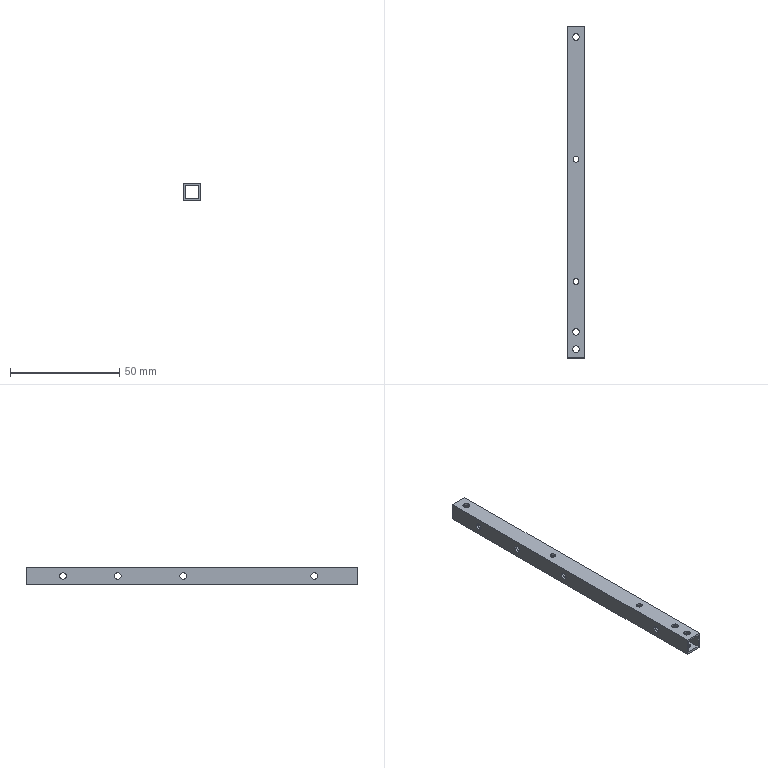Part | SolidWorks | features ICE 5, Extrusion 1 | 1 solid | 46 faces | box 8 x 152 x 8 mm | volume 4129 mm3 | cylinder 36 | plane 10 | commonest cylinder face diameters 3.1 x28 2.6 x8
STEP:
#1=CARTESIAN_POINT('',(1.3,35.,3.));
#2=VERTEX_POINT('',#1);
#3=CARTESIAN_POINT('',(-1.3,35.,3.));
#4=VERTEX_POINT('',#3);
#5=CARTESIAN_POINT('',(0.,35.,3.));
#6=DIRECTION('',(0.,0.,-1.));
#7=DIRECTION('',(-1.,0.,0.));
#8=AXIS2_PLACEMENT_3D('',#5,#6,#7);
#9=CIRCLE('',#8,1.3);
#10=EDGE_CURVE('',#2,#4,#9,.T.);
#11=ORIENTED_EDGE('',*,*,#10,.T.);
#12=CARTESIAN_POINT('',(-1.3,35.,4.));
#13=VERTEX_POINT('',#12);
#14=CARTESIAN_POINT('',(-1.3,35.,-6.));
#15=DIRECTION('',(0.,0.,1.));
#16=VECTOR('',#15,1000.);
#17=LINE('',#14,#16);
#18=EDGE_CURVE('',#4,#13,#17,.T.);
#19=ORIENTED_EDGE('',*,*,#18,.T.);
#20=CARTESIAN_POINT('',(1.3,35.,4.));
#21=VERTEX_POINT('',#20);
#22=CARTESIAN_POINT('',(0.,35.,4.));
#23=DIRECTION('',(0.,0.,1.));
#24=DIRECTION('',(1.,0.,0.));
#25=AXIS2_PLACEMENT_3D('',#22,#23,#24);
#26=CIRCLE('',#25,1.3);
#27=EDGE_CURVE('',#13,#21,#26,.T.);
#28=ORIENTED_EDGE('',*,*,#27,.T.);
#29=CARTESIAN_POINT('',(1.3,35.,-6.));
#30=DIRECTION('',(0.,0.,1.));
#31=VECTOR('',#30,1000.);
#32=LINE('',#29,#31);
#33=EDGE_CURVE('',#2,#21,#32,.T.);
#34=ORIENTED_EDGE('',*,*,#33,.F.);
#35=EDGE_LOOP('',(#11,#19,#28,#34));
#36=FACE_OUTER_BOUND('',#35,.T.);
#37=CARTESIAN_POINT('',(0.,35.,-6.));
#38=DIRECTION('',(0.,0.,1.));
#39=DIRECTION('',(1.,0.,0.));
#40=AXIS2_PLACEMENT_3D('',#37,#38,#39);
#41=CYLINDRICAL_SURFACE('',#40,1.3);
#42=ADVANCED_FACE('',(#36),#41,.F.);
#43=CARTESIAN_POINT('',(1.3,91.,3.));
#44=VERTEX_POINT('',#43);
#45=CARTESIAN_POINT('',(-1.3,91.,3.));
#46=VERTEX_POINT('',#45);
#47=CARTESIAN_POINT('',(0.,91.,3.));
#48=DIRECTION('',(0.,0.,-1.));
#49=DIRECTION('',(-1.,0.,0.));
#50=AXIS2_PLACEMENT_3D('',#47,#48,#49);
#51=CIRCLE('',#50,1.3);
#52=EDGE_CURVE('',#44,#46,#51,.T.);
#53=ORIENTED_EDGE('',*,*,#52,.T.);
#54=CARTESIAN_POINT('',(-1.3,91.,4.));
#55=VERTEX_POINT('',#54);
#56=CARTESIAN_POINT('',(-1.3,91.,-6.));
#57=DIRECTION('',(0.,0.,1.));
#58=VECTOR('',#57,1000.);
#59=LINE('',#56,#58);
#60=EDGE_CURVE('',#46,#55,#59,.T.);
#61=ORIENTED_EDGE('',*,*,#60,.T.);
#62=CARTESIAN_POINT('',(1.3,91.,4.));
#63=VERTEX_POINT('',#62);
#64=CARTESIAN_POINT('',(0.,91.,4.));
#65=DIRECTION('',(0.,0.,1.));
#66=DIRECTION('',(1.,0.,0.));
#67=AXIS2_PLACEMENT_3D('',#64,#65,#66);
#68=CIRCLE('',#67,1.3);
#69=EDGE_CURVE('',#55,#63,#68,.T.);
#70=ORIENTED_EDGE('',*,*,#69,.T.);
#71=CARTESIAN_POINT('',(1.3,91.,-6.));
#72=DIRECTION('',(0.,0.,1.));
#73=VECTOR('',#72,1000.);
#74=LINE('',#71,#73);
#75=EDGE_CURVE('',#44,#63,#74,.T.);
#76=ORIENTED_EDGE('',*,*,#75,.F.);
#77=EDGE_LOOP('',(#53,#61,#70,#76));
#78=FACE_OUTER_BOUND('',#77,.T.);
#79=CARTESIAN_POINT('',(0.,91.,-6.));
#80=DIRECTION('',(0.,0.,1.));
#81=DIRECTION('',(1.,0.,0.));
#82=AXIS2_PLACEMENT_3D('',#79,#80,#81);
#83=CYLINDRICAL_SURFACE('',#82,1.3);
#84=ADVANCED_FACE('',(#78),#83,.F.);
#85=CARTESIAN_POINT('',(-1.3,35.,-4.));
#86=VERTEX_POINT('',#85);
#87=CARTESIAN_POINT('',(1.3,35.,-4.));
#88=VERTEX_POINT('',#87);
#89=CARTESIAN_POINT('',(0.,35.,-4.));
#90=DIRECTION('',(0.,0.,1.));
#91=DIRECTION('',(1.,0.,0.));
#92=AXIS2_PLACEMENT_3D('',#89,#90,#91);
#93=CIRCLE('',#92,1.3);
#94=EDGE_CURVE('',#86,#88,#93,.T.);
#95=ORIENTED_EDGE('',*,*,#94,.F.);
#96=CARTESIAN_POINT('',(-1.3,35.,-3.));
#97=VERTEX_POINT('',#96);
#98=CARTESIAN_POINT('',(-1.3,35.,-6.));
#99=DIRECTION('',(0.,0.,1.));
#100=VECTOR('',#99,1000.);
#101=LINE('',#98,#100);
#102=EDGE_CURVE('',#86,#97,#101,.T.);
#103=ORIENTED_EDGE('',*,*,#102,.T.);
#104=CARTESIAN_POINT('',(1.3,35.,-3.));
#105=VERTEX_POINT('',#104);
#106=CARTESIAN_POINT('',(0.,35.,-3.));
#107=DIRECTION('',(0.,0.,1.));
#108=DIRECTION('',(1.,0.,0.));
#109=AXIS2_PLACEMENT_3D('',#106,#107,#108);
#110=CIRCLE('',#109,1.3);
#111=EDGE_CURVE('',#97,#105,#110,.T.);
#112=ORIENTED_EDGE('',*,*,#111,.T.);
#113=CARTESIAN_POINT('',(1.3,35.,-6.));
#114=DIRECTION('',(0.,0.,1.));
#115=VECTOR('',#114,1000.);
#116=LINE('',#113,#115);
#117=EDGE_CURVE('',#88,#105,#116,.T.);
#118=ORIENTED_EDGE('',*,*,#117,.F.);
#119=EDGE_LOOP('',(#95,#103,#112,#118));
#120=FACE_OUTER_BOUND('',#119,.T.);
#121=CARTESIAN_POINT('',(0.,35.,-6.));
#122=DIRECTION('',(0.,0.,1.));
#123=DIRECTION('',(1.,0.,0.));
#124=AXIS2_PLACEMENT_3D('',#121,#122,#123);
#125=CYLINDRICAL_SURFACE('',#124,1.3);
#126=ADVANCED_FACE('',(#120),#125,.F.);
#127=CARTESIAN_POINT('',(-1.3,91.,-4.));
#128=VERTEX_POINT('',#127);
#129=CARTESIAN_POINT('',(1.3,91.,-4.));
#130=VERTEX_POINT('',#129);
#131=CARTESIAN_POINT('',(0.,91.,-4.));
#132=DIRECTION('',(0.,0.,1.));
#133=DIRECTION('',(1.,0.,0.));
#134=AXIS2_PLACEMENT_3D('',#131,#132,#133);
#135=CIRCLE('',#134,1.3);
#136=EDGE_CURVE('',#128,#130,#135,.T.);
#137=ORIENTED_EDGE('',*,*,#136,.F.);
#138=CARTESIAN_POINT('',(-1.3,91.,-3.));
#139=VERTEX_POINT('',#138);
#140=CARTESIAN_POINT('',(-1.3,91.,-6.));
#141=DIRECTION('',(0.,0.,1.));
#142=VECTOR('',#141,1000.);
#143=LINE('',#140,#142);
#144=EDGE_CURVE('',#128,#139,#143,.T.);
#145=ORIENTED_EDGE('',*,*,#144,.T.);
#146=CARTESIAN_POINT('',(1.3,91.,-3.));
#147=VERTEX_POINT('',#146);
#148=CARTESIAN_POINT('',(0.,91.,-3.));
#149=DIRECTION('',(0.,0.,1.));
#150=DIRECTION('',(1.,0.,0.));
#151=AXIS2_PLACEMENT_3D('',#148,#149,#150);
#152=CIRCLE('',#151,1.3);
#153=EDGE_CURVE('',#139,#147,#152,.T.);
#154=ORIENTED_EDGE('',*,*,#153,.T.);
#155=CARTESIAN_POINT('',(1.3,91.,-6.));
#156=DIRECTION('',(0.,0.,1.));
#157=VECTOR('',#156,1000.);
#158=LINE('',#155,#157);
#159=EDGE_CURVE('',#130,#147,#158,.T.);
#160=ORIENTED_EDGE('',*,*,#159,.F.);
#161=EDGE_LOOP('',(#137,#145,#154,#160));
#162=FACE_OUTER_BOUND('',#161,.T.);
#163=CARTESIAN_POINT('',(0.,91.,-6.));
#164=DIRECTION('',(0.,0.,1.));
#165=DIRECTION('',(1.,0.,0.));
#166=AXIS2_PLACEMENT_3D('',#163,#164,#165);
#167=CYLINDRICAL_SURFACE('',#166,1.3);
#168=ADVANCED_FACE('',(#162),#167,.F.);
#169=CARTESIAN_POINT('',(-4.,135.,1.55));
#170=VERTEX_POINT('',#169);
#171=CARTESIAN_POINT('',(-4.,135.,-1.55));
#172=VERTEX_POINT('',#171);
#173=CARTESIAN_POINT('',(-4.,135.,0.));
#174=DIRECTION('',(1.,0.,0.));
#175=DIRECTION('',(0.,0.,-1.));
#176=AXIS2_PLACEMENT_3D('',#173,#174,#175);
#177=CIRCLE('',#176,1.55);
#178=EDGE_CURVE('',#170,#172,#177,.T.);
#179=ORIENTED_EDGE('',*,*,#178,.F.);
#180=CARTESIAN_POINT('',(-3.,135.,1.55));
#181=VERTEX_POINT('',#180);
#182=CARTESIAN_POINT('',(-4.,135.,1.55));
#183=DIRECTION('',(1.,0.,0.));
#184=VECTOR('',#183,1000.);
#185=LINE('',#182,#184);
#186=EDGE_CURVE('',#170,#181,#185,.T.);
#187=ORIENTED_EDGE('',*,*,#186,.T.);
#188=CARTESIAN_POINT('',(-3.,135.,-1.55));
#189=VERTEX_POINT('',#188);
#190=CARTESIAN_POINT('',(-3.,135.,0.));
#191=DIRECTION('',(1.,0.,0.));
#192=DIRECTION('',(0.,0.,-1.));
#193=AXIS2_PLACEMENT_3D('',#190,#191,#192);
#194=CIRCLE('',#193,1.55);
#195=EDGE_CURVE('',#181,#189,#194,.T.);
#196=ORIENTED_EDGE('',*,*,#195,.T.);
#197=CARTESIAN_POINT('',(-4.,135.,-1.55));
#198=DIRECTION('',(1.,0.,0.));
#199=VECTOR('',#198,1000.);
#200=LINE('',#197,#199);
#201=EDGE_CURVE('',#172,#189,#200,.T.);
#202=ORIENTED_EDGE('',*,*,#201,.F.);
#203=EDGE_LOOP('',(#179,#187,#196,#202));
#204=FACE_OUTER_BOUND('',#203,.T.);
#205=CARTESIAN_POINT('',(-4.,135.,0.));
#206=DIRECTION('',(1.,0.,0.));
#207=DIRECTION('',(0.,0.,-1.));
#208=AXIS2_PLACEMENT_3D('',#205,#206,#207);
#209=CYLINDRICAL_SURFACE('',#208,1.55);
#210=ADVANCED_FACE('',(#204),#209,.F.);
#211=CARTESIAN_POINT('',(-4.,80.,1.55));
#212=VERTEX_POINT('',#211);
#213=CARTESIAN_POINT('',(-4.,80.,-1.55));
#214=VERTEX_POINT('',#213);
#215=CARTESIAN_POINT('',(-4.,80.,0.));
#216=DIRECTION('',(1.,0.,0.));
#217=DIRECTION('',(0.,0.,-1.));
#218=AXIS2_PLACEMENT_3D('',#215,#216,#217);
#219=CIRCLE('',#218,1.55);
#220=EDGE_CURVE('',#212,#214,#219,.T.);
#221=ORIENTED_EDGE('',*,*,#220,.F.);
#222=CARTESIAN_POINT('',(-3.,80.,1.55));
#223=VERTEX_POINT('',#222);
#224=CARTESIAN_POINT('',(-4.,80.,1.55));
#225=DIRECTION('',(1.,0.,0.));
#226=VECTOR('',#225,1000.);
#227=LINE('',#224,#226);
#228=EDGE_CURVE('',#212,#223,#227,.T.);
#229=ORIENTED_EDGE('',*,*,#228,.T.);
#230=CARTESIAN_POINT('',(-3.,80.,-1.55));
#231=VERTEX_POINT('',#230);
#232=CARTESIAN_POINT('',(-3.,80.,0.));
#233=DIRECTION('',(1.,0.,0.));
#234=DIRECTION('',(0.,0.,-1.));
#235=AXIS2_PLACEMENT_3D('',#232,#233,#234);
#236=CIRCLE('',#235,1.55);
#237=EDGE_CURVE('',#223,#231,#236,.T.);
#238=ORIENTED_EDGE('',*,*,#237,.T.);
#239=CARTESIAN_POINT('',(-4.,80.,-1.55));
#240=DIRECTION('',(1.,0.,0.));
#241=VECTOR('',#240,1000.);
#242=LINE('',#239,#241);
#243=EDGE_CURVE('',#214,#231,#242,.T.);
#244=ORIENTED_EDGE('',*,*,#243,.F.);
#245=EDGE_LOOP('',(#221,#229,#238,#244));
#246=FACE_OUTER_BOUND('',#245,.T.);
#247=CARTESIAN_POINT('',(-4.,80.,0.));
#248=DIRECTION('',(1.,0.,0.));
#249=DIRECTION('',(0.,0.,-1.));
#250=AXIS2_PLACEMENT_3D('',#247,#248,#249);
#251=CYLINDRICAL_SURFACE('',#250,1.55);
#252=ADVANCED_FACE('',(#246),#251,.F.);
#253=CARTESIAN_POINT('',(-4.,110.,1.55));
#254=VERTEX_POINT('',#253);
#255=CARTESIAN_POINT('',(-4.,110.,-1.55));
#256=VERTEX_POINT('',#255);
#257=CARTESIAN_POINT('',(-4.,110.,0.));
#258=DIRECTION('',(1.,0.,0.));
#259=DIRECTION('',(0.,0.,-1.));
#260=AXIS2_PLACEMENT_3D('',#257,#258,#259);
#261=CIRCLE('',#260,1.55);
#262=EDGE_CURVE('',#254,#256,#261,.T.);
#263=ORIENTED_EDGE('',*,*,#262,.F.);
#264=CARTESIAN_POINT('',(-3.,110.,1.55));
#265=VERTEX_POINT('',#264);
#266=CARTESIAN_POINT('',(-4.,110.,1.55));
#267=DIRECTION('',(1.,0.,0.));
#268=VECTOR('',#267,1000.);
#269=LINE('',#266,#268);
#270=EDGE_CURVE('',#254,#265,#269,.T.);
#271=ORIENTED_EDGE('',*,*,#270,.T.);
#272=CARTESIAN_POINT('',(-3.,110.,-1.55));
#273=VERTEX_POINT('',#272);
#274=CARTESIAN_POINT('',(-3.,110.,0.));
#275=DIRECTION('',(1.,0.,0.));
#276=DIRECTION('',(0.,0.,-1.));
#277=AXIS2_PLACEMENT_3D('',#274,#275,#276);
#278=CIRCLE('',#277,1.55);
#279=EDGE_CURVE('',#265,#273,#278,.T.);
#280=ORIENTED_EDGE('',*,*,#279,.T.);
#281=CARTESIAN_POINT('',(-4.,110.,-1.55));
#282=DIRECTION('',(1.,0.,0.));
#283=VECTOR('',#282,1000.);
#284=LINE('',#281,#283);
#285=EDGE_CURVE('',#256,#273,#284,.T.);
#286=ORIENTED_EDGE('',*,*,#285,.F.);
#287=EDGE_LOOP('',(#263,#271,#280,#286));
#288=FACE_OUTER_BOUND('',#287,.T.);
#289=CARTESIAN_POINT('',(-4.,110.,0.));
#290=DIRECTION('',(1.,0.,0.));
#291=DIRECTION('',(0.,0.,-1.));
#292=AXIS2_PLACEMENT_3D('',#289,#290,#291);
#293=CYLINDRICAL_SURFACE('',#292,1.55);
#294=ADVANCED_FACE('',(#288),#293,.F.);
#295=CARTESIAN_POINT('',(-4.,20.,1.55));
#296=VERTEX_POINT('',#295);
#297=CARTESIAN_POINT('',(-4.,20.,-1.55));
#298=VERTEX_POINT('',#297);
#299=CARTESIAN_POINT('',(-4.,20.,0.));
#300=DIRECTION('',(1.,0.,0.));
#301=DIRECTION('',(0.,0.,-1.));
#302=AXIS2_PLACEMENT_3D('',#299,#300,#301);
#303=CIRCLE('',#302,1.55);
#304=EDGE_CURVE('',#296,#298,#303,.T.);
#305=ORIENTED_EDGE('',*,*,#304,.F.);
#306=CARTESIAN_POINT('',(-3.,20.,1.55));
#307=VERTEX_POINT('',#306);
#308=CARTESIAN_POINT('',(-4.,20.,1.55));
#309=DIRECTION('',(1.,0.,0.));
#310=VECTOR('',#309,1000.);
#311=LINE('',#308,#310);
#312=EDGE_CURVE('',#296,#307,#311,.T.);
#313=ORIENTED_EDGE('',*,*,#312,.T.);
#314=CARTESIAN_POINT('',(-3.,20.,-1.55));
#315=VERTEX_POINT('',#314);
#316=CARTESIAN_POINT('',(-3.,20.,0.));
#317=DIRECTION('',(1.,0.,0.));
#318=DIRECTION('',(0.,0.,-1.));
#319=AXIS2_PLACEMENT_3D('',#316,#317,#318);
#320=CIRCLE('',#319,1.55);
#321=EDGE_CURVE('',#307,#315,#320,.T.);
#322=ORIENTED_EDGE('',*,*,#321,.T.);
#323=CARTESIAN_POINT('',(-4.,20.,-1.55));
#324=DIRECTION('',(1.,0.,0.));
#325=VECTOR('',#324,1000.);
#326=LINE('',#323,#325);
#327=EDGE_CURVE('',#298,#315,#326,.T.);
#328=ORIENTED_EDGE('',*,*,#327,.F.);
#329=EDGE_LOOP('',(#305,#313,#322,#328));
#330=FACE_OUTER_BOUND('',#329,.T.);
#331=CARTESIAN_POINT('',(-4.,20.,0.));
#332=DIRECTION('',(1.,0.,0.));
#333=DIRECTION('',(0.,0.,-1.));
#334=AXIS2_PLACEMENT_3D('',#331,#332,#333);
#335=CYLINDRICAL_SURFACE('',#334,1.55);
#336=ADVANCED_FACE('',(#330),#335,.F.);
#337=CARTESIAN_POINT('',(3.,135.,-1.55));
#338=VERTEX_POINT('',#337);
#339=CARTESIAN_POINT('',(3.,135.,1.55));
#340=VERTEX_POINT('',#339);
#341=CARTESIAN_POINT('',(3.,135.,0.));
#342=DIRECTION('',(-1.,0.,0.));
#343=DIRECTION('',(0.,0.,1.));
#344=AXIS2_PLACEMENT_3D('',#341,#342,#343);
#345=CIRCLE('',#344,1.55);
#346=EDGE_CURVE('',#338,#340,#345,.T.);
#347=ORIENTED_EDGE('',*,*,#346,.T.);
#348=CARTESIAN_POINT('',(4.,135.,1.55));
#349=VERTEX_POINT('',#348);
#350=CARTESIAN_POINT('',(-4.,135.,1.55));
#351=DIRECTION('',(1.,0.,0.));
#352=VECTOR('',#351,1000.);
#353=LINE('',#350,#352);
#354=EDGE_CURVE('',#340,#349,#353,.T.);
#355=ORIENTED_EDGE('',*,*,#354,.T.);
#356=CARTESIAN_POINT('',(4.,135.,-1.55));
#357=VERTEX_POINT('',#356);
#358=CARTESIAN_POINT('',(4.,135.,0.));
#359=DIRECTION('',(1.,0.,0.));
#360=DIRECTION('',(0.,0.,-1.));
#361=AXIS2_PLACEMENT_3D('',#358,#359,#360);
#362=CIRCLE('',#361,1.55);
#363=EDGE_CURVE('',#349,#357,#362,.T.);
#364=ORIENTED_EDGE('',*,*,#363,.T.);
#365=CARTESIAN_POINT('',(-4.,135.,-1.55));
#366=DIRECTION('',(1.,0.,0.));
#367=VECTOR('',#366,1000.);
#368=LINE('',#365,#367);
#369=EDGE_CURVE('',#338,#357,#368,.T.);
#370=ORIENTED_EDGE('',*,*,#369,.F.);
#371=EDGE_LOOP('',(#347,#355,#364,#370));
#372=FACE_OUTER_BOUND('',#371,.T.);
#373=CARTESIAN_POINT('',(-4.,135.,0.));
#374=DIRECTION('',(1.,0.,0.));
#375=DIRECTION('',(0.,0.,-1.));
#376=AXIS2_PLACEMENT_3D('',#373,#374,#375);
#377=CYLINDRICAL_SURFACE('',#376,1.55);
#378=ADVANCED_FACE('',(#372),#377,.F.);
#379=CARTESIAN_POINT('',(3.,80.,-1.55));
#380=VERTEX_POINT('',#379);
#381=CARTESIAN_POINT('',(3.,80.,1.55));
#382=VERTEX_POINT('',#381);
#383=CARTESIAN_POINT('',(3.,80.,0.));
#384=DIRECTION('',(-1.,0.,0.));
#385=DIRECTION('',(0.,0.,1.));
#386=AXIS2_PLACEMENT_3D('',#383,#384,#385);
#387=CIRCLE('',#386,1.55);
#388=EDGE_CURVE('',#380,#382,#387,.T.);
#389=ORIENTED_EDGE('',*,*,#388,.T.);
#390=CARTESIAN_POINT('',(4.,80.,1.55));
#391=VERTEX_POINT('',#390);
#392=CARTESIAN_POINT('',(-4.,80.,1.55));
#393=DIRECTION('',(1.,0.,0.));
#394=VECTOR('',#393,1000.);
#395=LINE('',#392,#394);
#396=EDGE_CURVE('',#382,#391,#395,.T.);
#397=ORIENTED_EDGE('',*,*,#396,.T.);
#398=CARTESIAN_POINT('',(4.,80.,-1.55));
#399=VERTEX_POINT('',#398);
#400=CARTESIAN_POINT('',(4.,80.,0.));
#401=DIRECTION('',(1.,0.,0.));
#402=DIRECTION('',(0.,0.,-1.));
#403=AXIS2_PLACEMENT_3D('',#400,#401,#402);
#404=CIRCLE('',#403,1.55);
#405=EDGE_CURVE('',#391,#399,#404,.T.);
#406=ORIENTED_EDGE('',*,*,#405,.T.);
#407=CARTESIAN_POINT('',(-4.,80.,-1.55));
#408=DIRECTION('',(1.,0.,0.));
#409=VECTOR('',#408,1000.);
#410=LINE('',#407,#409);
#411=EDGE_CURVE('',#380,#399,#410,.T.);
#412=ORIENTED_EDGE('',*,*,#411,.F.);
#413=EDGE_LOOP('',(#389,#397,#406,#412));
#414=FACE_OUTER_BOUND('',#413,.T.);
#415=CARTESIAN_POINT('',(-4.,80.,0.));
#416=DIRECTION('',(1.,0.,0.));
#417=DIRECTION('',(0.,0.,-1.));
#418=AXIS2_PLACEMENT_3D('',#415,#416,#417);
#419=CYLINDRICAL_SURFACE('',#418,1.55);
#420=ADVANCED_FACE('',(#414),#419,.F.);
#421=CARTESIAN_POINT('',(3.,110.,-1.55));
#422=VERTEX_POINT('',#421);
#423=CARTESIAN_POINT('',(3.,110.,1.55));
#424=VERTEX_POINT('',#423);
#425=CARTESIAN_POINT('',(3.,110.,0.));
#426=DIRECTION('',(-1.,0.,0.));
#427=DIRECTION('',(0.,0.,1.));
#428=AXIS2_PLACEMENT_3D('',#425,#426,#427);
#429=CIRCLE('',#428,1.55);
#430=EDGE_CURVE('',#422,#424,#429,.T.);
#431=ORIENTED_EDGE('',*,*,#430,.T.);
#432=CARTESIAN_POINT('',(4.,110.,1.55));
#433=VERTEX_POINT('',#432);
#434=CARTESIAN_POINT('',(-4.,110.,1.55));
#435=DIRECTION('',(1.,0.,0.));
#436=VECTOR('',#435,1000.);
#437=LINE('',#434,#436);
#438=EDGE_CURVE('',#424,#433,#437,.T.);
#439=ORIENTED_EDGE('',*,*,#438,.T.);
#440=CARTESIAN_POINT('',(4.,110.,-1.55));
#441=VERTEX_POINT('',#440);
#442=CARTESIAN_POINT('',(4.,110.,0.));
#443=DIRECTION('',(1.,0.,0.));
#444=DIRECTION('',(0.,0.,-1.));
#445=AXIS2_PLACEMENT_3D('',#442,#443,#444);
#446=CIRCLE('',#445,1.55);
#447=EDGE_CURVE('',#433,#441,#446,.T.);
#448=ORIENTED_EDGE('',*,*,#447,.T.);
#449=CARTESIAN_POINT('',(-4.,110.,-1.55));
#450=DIRECTION('',(1.,0.,0.));
#451=VECTOR('',#450,1000.);
#452=LINE('',#449,#451);
#453=EDGE_CURVE('',#422,#441,#452,.T.);
#454=ORIENTED_EDGE('',*,*,#453,.F.);
#455=EDGE_LOOP('',(#431,#439,#448,#454));
#456=FACE_OUTER_BOUND('',#455,.T.);
#457=CARTESIAN_POINT('',(-4.,110.,0.));
#458=DIRECTION('',(1.,0.,0.));
#459=DIRECTION('',(0.,0.,-1.));
#460=AXIS2_PLACEMENT_3D('',#457,#458,#459);
#461=CYLINDRICAL_SURFACE('',#460,1.55);
#462=ADVANCED_FACE('',(#456),#461,.F.);
#463=CARTESIAN_POINT('',(3.,20.,-1.55));
#464=VERTEX_POINT('',#463);
#465=CARTESIAN_POINT('',(3.,20.,1.55));
#466=VERTEX_POINT('',#465);
#467=CARTESIAN_POINT('',(3.,20.,0.));
#468=DIRECTION('',(-1.,0.,0.));
#469=DIRECTION('',(0.,0.,1.));
#470=AXIS2_PLACEMENT_3D('',#467,#468,#469);
#471=CIRCLE('',#470,1.55);
#472=EDGE_CURVE('',#464,#466,#471,.T.);
#473=ORIENTED_EDGE('',*,*,#472,.T.);
#474=CARTESIAN_POINT('',(4.,20.,1.55));
#475=VERTEX_POINT('',#474);
#476=CARTESIAN_POINT('',(-4.,20.,1.55));
#477=DIRECTION('',(1.,0.,0.));
#478=VECTOR('',#477,1000.);
#479=LINE('',#476,#478);
#480=EDGE_CURVE('',#466,#475,#479,.T.);
#481=ORIENTED_EDGE('',*,*,#480,.T.);
#482=CARTESIAN_POINT('',(4.,20.,-1.55));
#483=VERTEX_POINT('',#482);
#484=CARTESIAN_POINT('',(4.,20.,0.));
#485=DIRECTION('',(1.,0.,0.));
#486=DIRECTION('',(0.,0.,-1.));
#487=AXIS2_PLACEMENT_3D('',#484,#485,#486);
#488=CIRCLE('',#487,1.55);
#489=EDGE_CURVE('',#475,#483,#488,.T.);
#490=ORIENTED_EDGE('',*,*,#489,.T.);
#491=CARTESIAN_POINT('',(-4.,20.,-1.55));
#492=DIRECTION('',(1.,0.,0.));
#493=VECTOR('',#492,1000.);
#494=LINE('',#491,#493);
#495=EDGE_CURVE('',#464,#483,#494,.T.);
#496=ORIENTED_EDGE('',*,*,#495,.F.);
#497=EDGE_LOOP('',(#473,#481,#490,#496));
#498=FACE_OUTER_BOUND('',#497,.T.);
#499=CARTESIAN_POINT('',(-4.,20.,0.));
#500=DIRECTION('',(1.,0.,0.));
#501=DIRECTION('',(0.,0.,-1.));
#502=AXIS2_PLACEMENT_3D('',#499,#500,#501);
#503=CYLINDRICAL_SURFACE('',#502,1.55);
#504=ADVANCED_FACE('',(#498),#503,.F.);
#505=CARTESIAN_POINT('',(1.55,147.,3.));
#506=VERTEX_POINT('',#505);
#507=CARTESIAN_POINT('',(-1.55,147.,3.));
#508=VERTEX_POINT('',#507);
#509=CARTESIAN_POINT('',(0.,147.,3.));
#510=DIRECTION('',(0.,0.,-1.));
#511=DIRECTION('',(-1.,0.,0.));
#512=AXIS2_PLACEMENT_3D('',#509,#510,#511);
#513=CIRCLE('',#512,1.55);
#514=EDGE_CURVE('',#506,#508,#513,.T.);
#515=ORIENTED_EDGE('',*,*,#514,.T.);
#516=CARTESIAN_POINT('',(-1.55,147.,4.));
#517=VERTEX_POINT('',#516);
#518=CARTESIAN_POINT('',(-1.55,147.,-4.));
#519=DIRECTION('',(0.,0.,1.));
#520=VECTOR('',#519,1000.);
#521=LINE('',#518,#520);
#522=EDGE_CURVE('',#508,#517,#521,.T.);
#523=ORIENTED_EDGE('',*,*,#522,.T.);
#524=CARTESIAN_POINT('',(1.55,147.,4.));
#525=VERTEX_POINT('',#524);
#526=CARTESIAN_POINT('',(0.,147.,4.));
#527=DIRECTION('',(0.,0.,1.));
#528=DIRECTION('',(1.,0.,0.));
#529=AXIS2_PLACEMENT_3D('',#526,#527,#528);
#530=CIRCLE('',#529,1.55);
#531=EDGE_CURVE('',#517,#525,#530,.T.);
#532=ORIENTED_EDGE('',*,*,#531,.T.);
#533=CARTESIAN_POINT('',(1.55,147.,-4.));
#534=DIRECTION('',(0.,0.,1.));
#535=VECTOR('',#534,1000.);
#536=LINE('',#533,#535);
#537=EDGE_CURVE('',#506,#525,#536,.T.);
#538=ORIENTED_EDGE('',*,*,#537,.F.);
#539=EDGE_LOOP('',(#515,#523,#532,#538));
#540=FACE_OUTER_BOUND('',#539,.T.);
#541=CARTESIAN_POINT('',(0.,147.,-4.));
#542=DIRECTION('',(0.,0.,1.));
#543=DIRECTION('',(1.,0.,0.));
#544=AXIS2_PLACEMENT_3D('',#541,#542,#543);
#545=CYLINDRICAL_SURFACE('',#544,1.55);
#546=ADVANCED_FACE('',(#540),#545,.F.);
#547=CARTESIAN_POINT('',(1.55,4.,3.));
#548=VERTEX_POINT('',#547);
#549=CARTESIAN_POINT('',(-1.55,4.,3.));
#550=VERTEX_POINT('',#549);
#551=CARTESIAN_POINT('',(0.,4.,3.));
#552=DIRECTION('',(0.,0.,-1.));
#553=DIRECTION('',(-1.,0.,0.));
#554=AXIS2_PLACEMENT_3D('',#551,#552,#553);
#555=CIRCLE('',#554,1.55);
#556=EDGE_CURVE('',#548,#550,#555,.T.);
#557=ORIENTED_EDGE('',*,*,#556,.T.);
#558=CARTESIAN_POINT('',(-1.55,4.,4.));
#559=VERTEX_POINT('',#558);
#560=CARTESIAN_POINT('',(-1.55,4.,-4.));
#561=DIRECTION('',(0.,0.,1.));
#562=VECTOR('',#561,1000.);
#563=LINE('',#560,#562);
#564=EDGE_CURVE('',#550,#559,#563,.T.);
#565=ORIENTED_EDGE('',*,*,#564,.T.);
#566=CARTESIAN_POINT('',(1.55,4.,4.));
#567=VERTEX_POINT('',#566);
#568=CARTESIAN_POINT('',(0.,4.,4.));
#569=DIRECTION('',(0.,0.,1.));
#570=DIRECTION('',(1.,0.,0.));
#571=AXIS2_PLACEMENT_3D('',#568,#569,#570);
#572=CIRCLE('',#571,1.55);
#573=EDGE_CURVE('',#559,#567,#572,.T.);
#574=ORIENTED_EDGE('',*,*,#573,.T.);
#575=CARTESIAN_POINT('',(1.55,4.,-4.));
#576=DIRECTION('',(0.,0.,1.));
#577=VECTOR('',#576,1000.);
#578=LINE('',#575,#577);
#579=EDGE_CURVE('',#548,#567,#578,.T.);
#580=ORIENTED_EDGE('',*,*,#579,.F.);
#581=EDGE_LOOP('',(#557,#565,#574,#580));
#582=FACE_OUTER_BOUND('',#581,.T.);
#583=CARTESIAN_POINT('',(0.,4.,-4.));
#584=DIRECTION('',(0.,0.,1.));
#585=DIRECTION('',(1.,0.,0.));
#586=AXIS2_PLACEMENT_3D('',#583,#584,#585);
#587=CYLINDRICAL_SURFACE('',#586,1.55);
#588=ADVANCED_FACE('',(#582),#587,.F.);
#589=CARTESIAN_POINT('',(1.55,12.,3.));
#590=VERTEX_POINT('',#589);
#591=CARTESIAN_POINT('',(-1.55,12.,3.));
#592=VERTEX_POINT('',#591);
#593=CARTESIAN_POINT('',(0.,12.,3.));
#594=DIRECTION('',(0.,0.,-1.));
#595=DIRECTION('',(-1.,0.,0.));
#596=AXIS2_PLACEMENT_3D('',#593,#594,#595);
#597=CIRCLE('',#596,1.55);
#598=EDGE_CURVE('',#590,#592,#597,.T.);
#599=ORIENTED_EDGE('',*,*,#598,.T.);
#600=CARTESIAN_POINT('',(-1.55,12.,4.));
#601=VERTEX_POINT('',#600);
#602=CARTESIAN_POINT('',(-1.55,12.,-4.));
#603=DIRECTION('',(0.,0.,1.));
#604=VECTOR('',#603,1000.);
#605=LINE('',#602,#604);
#606=EDGE_CURVE('',#592,#601,#605,.T.);
#607=ORIENTED_EDGE('',*,*,#606,.T.);
#608=CARTESIAN_POINT('',(1.55,12.,4.));
#609=VERTEX_POINT('',#608);
#610=CARTESIAN_POINT('',(0.,12.,4.));
#611=DIRECTION('',(0.,0.,1.));
#612=DIRECTION('',(1.,0.,0.));
#613=AXIS2_PLACEMENT_3D('',#610,#611,#612);
#614=CIRCLE('',#613,1.55);
#615=EDGE_CURVE('',#601,#609,#614,.T.);
#616=ORIENTED_EDGE('',*,*,#615,.T.);
#617=CARTESIAN_POINT('',(1.55,12.,-4.));
#618=DIRECTION('',(0.,0.,1.));
#619=VECTOR('',#618,1000.);
#620=LINE('',#617,#619);
#621=EDGE_CURVE('',#590,#609,#620,.T.);
#622=ORIENTED_EDGE('',*,*,#621,.F.);
#623=EDGE_LOOP('',(#599,#607,#616,#622));
#624=FACE_OUTER_BOUND('',#623,.T.);
#625=CARTESIAN_POINT('',(0.,12.,-4.));
#626=DIRECTION('',(0.,0.,1.));
#627=DIRECTION('',(1.,0.,0.));
#628=AXIS2_PLACEMENT_3D('',#625,#626,#627);
#629=CYLINDRICAL_SURFACE('',#628,1.55);
#630=ADVANCED_FACE('',(#624),#629,.F.);
#631=CARTESIAN_POINT('',(-1.55,147.,-4.));
#632=VERTEX_POINT('',#631);
#633=CARTESIAN_POINT('',(1.55,147.,-4.));
#634=VERTEX_POINT('',#633);
#635=CARTESIAN_POINT('',(0.,147.,-4.));
#636=DIRECTION('',(0.,0.,1.));
#637=DIRECTION('',(1.,0.,0.));
#638=AXIS2_PLACEMENT_3D('',#635,#636,#637);
#639=CIRCLE('',#638,1.55);
#640=EDGE_CURVE('',#632,#634,#639,.T.);
#641=ORIENTED_EDGE('',*,*,#640,.F.);
#642=CARTESIAN_POINT('',(-1.55,147.,-3.));
#643=VERTEX_POINT('',#642);
#644=CARTESIAN_POINT('',(-1.55,147.,-4.));
#645=DIRECTION('',(0.,0.,1.));
#646=VECTOR('',#645,1000.);
#647=LINE('',#644,#646);
#648=EDGE_CURVE('',#632,#643,#647,.T.);
#649=ORIENTED_EDGE('',*,*,#648,.T.);
#650=CARTESIAN_POINT('',(1.55,147.,-3.));
#651=VERTEX_POINT('',#650);
#652=CARTESIAN_POINT('',(0.,147.,-3.));
#653=DIRECTION('',(0.,0.,1.));
#654=DIRECTION('',(1.,0.,0.));
#655=AXIS2_PLACEMENT_3D('',#652,#653,#654);
#656=CIRCLE('',#655,1.55);
#657=EDGE_CURVE('',#643,#651,#656,.T.);
#658=ORIENTED_EDGE('',*,*,#657,.T.);
#659=CARTESIAN_POINT('',(1.55,147.,-4.));
#660=DIRECTION('',(0.,0.,1.));
#661=VECTOR('',#660,1000.);
#662=LINE('',#659,#661);
#663=EDGE_CURVE('',#634,#651,#662,.T.);
#664=ORIENTED_EDGE('',*,*,#663,.F.);
#665=EDGE_LOOP('',(#641,#649,#658,#664));
#666=FACE_OUTER_BOUND('',#665,.T.);
#667=CARTESIAN_POINT('',(0.,147.,-4.));
#668=DIRECTION('',(0.,0.,1.));
#669=DIRECTION('',(1.,0.,0.));
#670=AXIS2_PLACEMENT_3D('',#667,#668,#669);
#671=CYLINDRICAL_SURFACE('',#670,1.55);
#672=ADVANCED_FACE('',(#666),#671,.F.);
#673=CARTESIAN_POINT('',(-1.55,4.,-4.));
#674=VERTEX_POINT('',#673);
#675=CARTESIAN_POINT('',(1.55,4.,-4.));
#676=VERTEX_POINT('',#675);
#677=CARTESIAN_POINT('',(0.,4.,-4.));
#678=DIRECTION('',(0.,0.,1.));
#679=DIRECTION('',(1.,0.,0.));
#680=AXIS2_PLACEMENT_3D('',#677,#678,#679);
#681=CIRCLE('',#680,1.55);
#682=EDGE_CURVE('',#674,#676,#681,.T.);
#683=ORIENTED_EDGE('',*,*,#682,.F.);
#684=CARTESIAN_POINT('',(-1.55,4.,-3.));
#685=VERTEX_POINT('',#684);
#686=CARTESIAN_POINT('',(-1.55,4.,-4.));
#687=DIRECTION('',(0.,0.,1.));
#688=VECTOR('',#687,1000.);
#689=LINE('',#686,#688);
#690=EDGE_CURVE('',#674,#685,#689,.T.);
#691=ORIENTED_EDGE('',*,*,#690,.T.);
#692=CARTESIAN_POINT('',(1.55,4.,-3.));
#693=VERTEX_POINT('',#692);
#694=CARTESIAN_POINT('',(0.,4.,-3.));
#695=DIRECTION('',(0.,0.,1.));
#696=DIRECTION('',(1.,0.,0.));
#697=AXIS2_PLACEMENT_3D('',#694,#695,#696);
#698=CIRCLE('',#697,1.55);
#699=EDGE_CURVE('',#685,#693,#698,.T.);
#700=ORIENTED_EDGE('',*,*,#699,.T.);
#701=CARTESIAN_POINT('',(1.55,4.,-4.));
#702=DIRECTION('',(0.,0.,1.));
#703=VECTOR('',#702,1000.);
#704=LINE('',#701,#703);
#705=EDGE_CURVE('',#676,#693,#704,.T.);
#706=ORIENTED_EDGE('',*,*,#705,.F.);
#707=EDGE_LOOP('',(#683,#691,#700,#706));
#708=FACE_OUTER_BOUND('',#707,.T.);
#709=CARTESIAN_POINT('',(0.,4.,-4.));
#710=DIRECTION('',(0.,0.,1.));
#711=DIRECTION('',(1.,0.,0.));
#712=AXIS2_PLACEMENT_3D('',#709,#710,#711);
#713=CYLINDRICAL_SURFACE('',#712,1.55);
#714=ADVANCED_FACE('',(#708),#713,.F.);
#715=CARTESIAN_POINT('',(-1.55,12.,-4.));
#716=VERTEX_POINT('',#715);
#717=CARTESIAN_POINT('',(1.55,12.,-4.));
#718=VERTEX_POINT('',#717);
#719=CARTESIAN_POINT('',(0.,12.,-4.));
#720=DIRECTION('',(0.,0.,1.));
#721=DIRECTION('',(1.,0.,0.));
#722=AXIS2_PLACEMENT_3D('',#719,#720,#721);
#723=CIRCLE('',#722,1.55);
#724=EDGE_CURVE('',#716,#718,#723,.T.);
#725=ORIENTED_EDGE('',*,*,#724,.F.);
#726=CARTESIAN_POINT('',(-1.55,12.,-3.));
#727=VERTEX_POINT('',#726);
#728=CARTESIAN_POINT('',(-1.55,12.,-4.));
#729=DIRECTION('',(0.,0.,1.));
#730=VECTOR('',#729,1000.);
#731=LINE('',#728,#730);
#732=EDGE_CURVE('',#716,#727,#731,.T.);
#733=ORIENTED_EDGE('',*,*,#732,.T.);
#734=CARTESIAN_POINT('',(1.55,12.,-3.));
#735=VERTEX_POINT('',#734);
#736=CARTESIAN_POINT('',(0.,12.,-3.));
#737=DIRECTION('',(0.,0.,1.));
#738=DIRECTION('',(1.,0.,0.));
#739=AXIS2_PLACEMENT_3D('',#736,#737,#738);
#740=CIRCLE('',#739,1.55);
#741=EDGE_CURVE('',#727,#735,#740,.T.);
#742=ORIENTED_EDGE('',*,*,#741,.T.);
#743=CARTESIAN_POINT('',(1.55,12.,-4.));
#744=DIRECTION('',(0.,0.,1.));
#745=VECTOR('',#744,1000.);
#746=LINE('',#743,#745);
#747=EDGE_CURVE('',#718,#735,#746,.T.);
#748=ORIENTED_EDGE('',*,*,#747,.F.);
#749=EDGE_LOOP('',(#725,#733,#742,#748));
#750=FACE_OUTER_BOUND('',#749,.T.);
#751=CARTESIAN_POINT('',(0.,12.,-4.));
#752=DIRECTION('',(0.,0.,1.));
#753=DIRECTION('',(1.,0.,0.));
#754=AXIS2_PLACEMENT_3D('',#751,#752,#753);
#755=CYLINDRICAL_SURFACE('',#754,1.55);
#756=ADVANCED_FACE('',(#750),#755,.F.);
#757=CARTESIAN_POINT('',(4.,152.,4.));
#758=VERTEX_POINT('',#757);
#759=CARTESIAN_POINT('',(4.,152.,-4.));
#760=VERTEX_POINT('',#759);
#761=CARTESIAN_POINT('',(4.,152.,-4.));
#762=DIRECTION('',(0.,0.,-1.));
#763=VECTOR('',#762,1000.);
#764=LINE('',#761,#763);
#765=EDGE_CURVE('',#758,#760,#764,.T.);
#766=ORIENTED_EDGE('',*,*,#765,.T.);
#767=CARTESIAN_POINT('',(-4.,152.,-4.));
#768=VERTEX_POINT('',#767);
#769=CARTESIAN_POINT('',(-4.,152.,-4.));
#770=DIRECTION('',(-1.,0.,0.));
#771=VECTOR('',#770,1000.);
#772=LINE('',#769,#771);
#773=EDGE_CURVE('',#760,#768,#772,.T.);
#774=ORIENTED_EDGE('',*,*,#773,.T.);
#775=CARTESIAN_POINT('',(-4.,152.,4.));
#776=VERTEX_POINT('',#775);
#777=CARTESIAN_POINT('',(-4.,152.,-4.));
#778=DIRECTION('',(0.,0.,1.));
#779=VECTOR('',#778,1000.);
#780=LINE('',#777,#779);
#781=EDGE_CURVE('',#768,#776,#780,.T.);
#782=ORIENTED_EDGE('',*,*,#781,.T.);
#783=CARTESIAN_POINT('',(-4.,152.,4.));
#784=DIRECTION('',(1.,0.,0.));
#785=VECTOR('',#784,1000.);
#786=LINE('',#783,#785);
#787=EDGE_CURVE('',#776,#758,#786,.T.);
#788=ORIENTED_EDGE('',*,*,#787,.T.);
#789=EDGE_LOOP('',(#766,#774,#782,#788));
#790=FACE_OUTER_BOUND('',#789,.T.);
#791=CARTESIAN_POINT('',(-3.,152.,3.));
#792=VERTEX_POINT('',#791);
#793=CARTESIAN_POINT('',(3.,152.,3.));
#794=VERTEX_POINT('',#793);
#795=CARTESIAN_POINT('',(-3.,152.,3.));
#796=DIRECTION('',(1.,0.,0.));
#797=VECTOR('',#796,1000.);
#798=LINE('',#795,#797);
#799=EDGE_CURVE('',#792,#794,#798,.T.);
#800=ORIENTED_EDGE('',*,*,#799,.F.);
#801=CARTESIAN_POINT('',(-3.,152.,-3.));
#802=VERTEX_POINT('',#801);
#803=CARTESIAN_POINT('',(-3.,152.,-3.));
#804=DIRECTION('',(0.,0.,1.));
#805=VECTOR('',#804,1000.);
#806=LINE('',#803,#805);
#807=EDGE_CURVE('',#802,#792,#806,.T.);
#808=ORIENTED_EDGE('',*,*,#807,.F.);
#809=CARTESIAN_POINT('',(3.,152.,-3.));
#810=VERTEX_POINT('',#809);
#811=CARTESIAN_POINT('',(-3.,152.,-3.));
#812=DIRECTION('',(-1.,0.,0.));
#813=VECTOR('',#812,1000.);
#814=LINE('',#811,#813);
#815=EDGE_CURVE('',#810,#802,#814,.T.);
#816=ORIENTED_EDGE('',*,*,#815,.F.);
#817=CARTESIAN_POINT('',(3.,152.,-3.));
#818=DIRECTION('',(0.,0.,-1.));
#819=VECTOR('',#818,1000.);
#820=LINE('',#817,#819);
#821=EDGE_CURVE('',#794,#810,#820,.T.);
#822=ORIENTED_EDGE('',*,*,#821,.F.);
#823=EDGE_LOOP('',(#800,#808,#816,#822));
#824=FACE_BOUND('',#823,.T.);
#825=CARTESIAN_POINT('',(0.,152.,0.));
#826=DIRECTION('',(0.,1.,0.));
#827=DIRECTION('',(0.,0.,1.));
#828=AXIS2_PLACEMENT_3D('',#825,#826,#827);
#829=PLANE('',#828);
#830=ADVANCED_FACE('',(#790,#824),#829,.T.);
#831=CARTESIAN_POINT('',(4.,0.,4.));
#832=VERTEX_POINT('',#831);
#833=CARTESIAN_POINT('',(4.,0.,-4.));
#834=VERTEX_POINT('',#833);
#835=CARTESIAN_POINT('',(4.,0.,-4.));
#836=DIRECTION('',(0.,0.,-1.));
#837=VECTOR('',#836,1000.);
#838=LINE('',#835,#837);
#839=EDGE_CURVE('',#832,#834,#838,.T.);
#840=ORIENTED_EDGE('',*,*,#839,.F.);
#841=CARTESIAN_POINT('',(-4.,0.,4.));
#842=VERTEX_POINT('',#841);
#843=CARTESIAN_POINT('',(-4.,0.,4.));
#844=DIRECTION('',(1.,0.,0.));
#845=VECTOR('',#844,1000.);
#846=LINE('',#843,#845);
#847=EDGE_CURVE('',#842,#832,#846,.T.);
#848=ORIENTED_EDGE('',*,*,#847,.F.);
#849=CARTESIAN_POINT('',(-4.,0.,-4.));
#850=VERTEX_POINT('',#849);
#851=CARTESIAN_POINT('',(-4.,0.,-4.));
#852=DIRECTION('',(0.,0.,1.));
#853=VECTOR('',#852,1000.);
#854=LINE('',#851,#853);
#855=EDGE_CURVE('',#850,#842,#854,.T.);
#856=ORIENTED_EDGE('',*,*,#855,.F.);
#857=CARTESIAN_POINT('',(-4.,0.,-4.));
#858=DIRECTION('',(-1.,0.,0.));
#859=VECTOR('',#858,1000.);
#860=LINE('',#857,#859);
#861=EDGE_CURVE('',#834,#850,#860,.T.);
#862=ORIENTED_EDGE('',*,*,#861,.F.);
#863=EDGE_LOOP('',(#840,#848,#856,#862));
#864=FACE_OUTER_BOUND('',#863,.T.);
#865=CARTESIAN_POINT('',(-3.,0.,-3.));
#866=VERTEX_POINT('',#865);
#867=CARTESIAN_POINT('',(-3.,0.,3.));
#868=VERTEX_POINT('',#867);
#869=CARTESIAN_POINT('',(-3.,0.,-3.));
#870=DIRECTION('',(0.,0.,1.));
#871=VECTOR('',#870,1000.);
#872=LINE('',#869,#871);
#873=EDGE_CURVE('',#866,#868,#872,.T.);
#874=ORIENTED_EDGE('',*,*,#873,.T.);
#875=CARTESIAN_POINT('',(3.,0.,3.));
#876=VERTEX_POINT('',#875);
#877=CARTESIAN_POINT('',(-3.,0.,3.));
#878=DIRECTION('',(1.,0.,0.));
#879=VECTOR('',#878,1000.);
#880=LINE('',#877,#879);
#881=EDGE_CURVE('',#868,#876,#880,.T.);
#882=ORIENTED_EDGE('',*,*,#881,.T.);
#883=CARTESIAN_POINT('',(3.,0.,-3.));
#884=VERTEX_POINT('',#883);
#885=CARTESIAN_POINT('',(3.,0.,-3.));
#886=DIRECTION('',(0.,0.,-1.));
#887=VECTOR('',#886,1000.);
#888=LINE('',#885,#887);
#889=EDGE_CURVE('',#876,#884,#888,.T.);
#890=ORIENTED_EDGE('',*,*,#889,.T.);
#891=CARTESIAN_POINT('',(-3.,0.,-3.));
#892=DIRECTION('',(-1.,0.,0.));
#893=VECTOR('',#892,1000.);
#894=LINE('',#891,#893);
#895=EDGE_CURVE('',#884,#866,#894,.T.);
#896=ORIENTED_EDGE('',*,*,#895,.T.);
#897=EDGE_LOOP('',(#874,#882,#890,#896));
#898=FACE_BOUND('',#897,.T.);
#899=CARTESIAN_POINT('',(0.,0.,0.));
#900=DIRECTION('',(0.,1.,0.));
#901=DIRECTION('',(0.,0.,1.));
#902=AXIS2_PLACEMENT_3D('',#899,#900,#901);
#903=PLANE('',#902);
#904=ADVANCED_FACE('',(#864,#898),#903,.F.);
#905=CARTESIAN_POINT('',(4.,135.,0.));
#906=DIRECTION('',(1.,0.,0.));
#907=DIRECTION('',(0.,0.,-1.));
#908=AXIS2_PLACEMENT_3D('',#905,#906,#907);
#909=CIRCLE('',#908,1.55);
#910=EDGE_CURVE('',#357,#349,#909,.T.);
#911=ORIENTED_EDGE('',*,*,#910,.F.);
#912=ORIENTED_EDGE('',*,*,#363,.F.);
#913=EDGE_LOOP('',(#911,#912));
#914=FACE_BOUND('',#913,.T.);
#915=CARTESIAN_POINT('',(4.,80.,0.));
#916=DIRECTION('',(1.,0.,0.));
#917=DIRECTION('',(0.,0.,-1.));
#918=AXIS2_PLACEMENT_3D('',#915,#916,#917);
#919=CIRCLE('',#918,1.55);
#920=EDGE_CURVE('',#399,#391,#919,.T.);
#921=ORIENTED_EDGE('',*,*,#920,.F.);
#922=ORIENTED_EDGE('',*,*,#405,.F.);
#923=EDGE_LOOP('',(#921,#922));
#924=FACE_BOUND('',#923,.T.);
#925=CARTESIAN_POINT('',(4.,110.,0.));
#926=DIRECTION('',(1.,0.,0.));
#927=DIRECTION('',(0.,0.,-1.));
#928=AXIS2_PLACEMENT_3D('',#925,#926,#927);
#929=CIRCLE('',#928,1.55);
#930=EDGE_CURVE('',#441,#433,#929,.T.);
#931=ORIENTED_EDGE('',*,*,#930,.F.);
#932=ORIENTED_EDGE('',*,*,#447,.F.);
#933=EDGE_LOOP('',(#931,#932));
#934=FACE_BOUND('',#933,.T.);
#935=CARTESIAN_POINT('',(4.,20.,0.));
#936=DIRECTION('',(1.,0.,0.));
#937=DIRECTION('',(0.,0.,-1.));
#938=AXIS2_PLACEMENT_3D('',#935,#936,#937);
#939=CIRCLE('',#938,1.55);
#940=EDGE_CURVE('',#483,#475,#939,.T.);
#941=ORIENTED_EDGE('',*,*,#940,.F.);
#942=ORIENTED_EDGE('',*,*,#489,.F.);
#943=EDGE_LOOP('',(#941,#942));
#944=FACE_BOUND('',#943,.T.);
#945=ORIENTED_EDGE('',*,*,#839,.T.);
#946=CARTESIAN_POINT('',(4.,152.,-4.));
#947=DIRECTION('',(0.,-1.,0.));
#948=VECTOR('',#947,1000.);
#949=LINE('',#946,#948);
#950=EDGE_CURVE('',#760,#834,#949,.T.);
#951=ORIENTED_EDGE('',*,*,#950,.F.);
#952=ORIENTED_EDGE('',*,*,#765,.F.);
#953=CARTESIAN_POINT('',(4.,152.,4.));
#954=DIRECTION('',(0.,-1.,0.));
#955=VECTOR('',#954,1000.);
#956=LINE('',#953,#955);
#957=EDGE_CURVE('',#758,#832,#956,.T.);
#958=ORIENTED_EDGE('',*,*,#957,.T.);
#959=EDGE_LOOP('',(#945,#951,#952,#958));
#960=FACE_OUTER_BOUND('',#959,.T.);
#961=CARTESIAN_POINT('',(4.,152.,-4.));
#962=DIRECTION('',(-1.,0.,0.));
#963=DIRECTION('',(0.,0.,1.));
#964=AXIS2_PLACEMENT_3D('',#961,#962,#963);
#965=PLANE('',#964);
#966=ADVANCED_FACE('',(#914,#924,#934,#944,#960),#965,.F.);
#967=CARTESIAN_POINT('',(0.,35.,-4.));
#968=DIRECTION('',(0.,0.,1.));
#969=DIRECTION('',(1.,0.,0.));
#970=AXIS2_PLACEMENT_3D('',#967,#968,#969);
#971=CIRCLE('',#970,1.3);
#972=EDGE_CURVE('',#88,#86,#971,.T.);
#973=ORIENTED_EDGE('',*,*,#972,.T.);
#974=ORIENTED_EDGE('',*,*,#94,.T.);
#975=EDGE_LOOP('',(#973,#974));
#976=FACE_BOUND('',#975,.T.);
#977=CARTESIAN_POINT('',(0.,91.,-4.));
#978=DIRECTION('',(0.,0.,1.));
#979=DIRECTION('',(1.,0.,0.));
#980=AXIS2_PLACEMENT_3D('',#977,#978,#979);
#981=CIRCLE('',#980,1.3);
#982=EDGE_CURVE('',#130,#128,#981,.T.);
#983=ORIENTED_EDGE('',*,*,#982,.T.);
#984=ORIENTED_EDGE('',*,*,#136,.T.);
#985=EDGE_LOOP('',(#983,#984));
#986=FACE_BOUND('',#985,.T.);
#987=CARTESIAN_POINT('',(0.,147.,-4.));
#988=DIRECTION('',(0.,0.,1.));
#989=DIRECTION('',(1.,0.,0.));
#990=AXIS2_PLACEMENT_3D('',#987,#988,#989);
#991=CIRCLE('',#990,1.55);
#992=EDGE_CURVE('',#634,#632,#991,.T.);
#993=ORIENTED_EDGE('',*,*,#992,.T.);
#994=ORIENTED_EDGE('',*,*,#640,.T.);
#995=EDGE_LOOP('',(#993,#994));
#996=FACE_BOUND('',#995,.T.);
#997=CARTESIAN_POINT('',(0.,4.,-4.));
#998=DIRECTION('',(0.,0.,1.));
#999=DIRECTION('',(1.,0.,0.));
#1000=AXIS2_PLACEMENT_3D('',#997,#998,#999);
#1001=CIRCLE('',#1000,1.55);
#1002=EDGE_CURVE('',#676,#674,#1001,.T.);
#1003=ORIENTED_EDGE('',*,*,#1002,.T.);
#1004=ORIENTED_EDGE('',*,*,#682,.T.);
#1005=EDGE_LOOP('',(#1003,#1004));
#1006=FACE_BOUND('',#1005,.T.);
#1007=CARTESIAN_POINT('',(0.,12.,-4.));
#1008=DIRECTION('',(0.,0.,1.));
#1009=DIRECTION('',(1.,0.,0.));
#1010=AXIS2_PLACEMENT_3D('',#1007,#1008,#1009);
#1011=CIRCLE('',#1010,1.55);
#1012=EDGE_CURVE('',#718,#716,#1011,.T.);
#1013=ORIENTED_EDGE('',*,*,#1012,.T.);
#1014=ORIENTED_EDGE('',*,*,#724,.T.);
#1015=EDGE_LOOP('',(#1013,#1014));
#1016=FACE_BOUND('',#1015,.T.);
#1017=ORIENTED_EDGE('',*,*,#861,.T.);
#1018=CARTESIAN_POINT('',(-4.,152.,-4.));
#1019=DIRECTION('',(0.,-1.,0.));
#1020=VECTOR('',#1019,1000.);
#1021=LINE('',#1018,#1020);
#1022=EDGE_CURVE('',#768,#850,#1021,.T.);
#1023=ORIENTED_EDGE('',*,*,#1022,.F.);
#1024=ORIENTED_EDGE('',*,*,#773,.F.);
#1025=ORIENTED_EDGE('',*,*,#950,.T.);
#1026=EDGE_LOOP('',(#1017,#1023,#1024,#1025));
#1027=FACE_OUTER_BOUND('',#1026,.T.);
#1028=CARTESIAN_POINT('',(-4.,152.,-4.));
#1029=DIRECTION('',(0.,0.,1.));
#1030=DIRECTION('',(1.,0.,0.));
#1031=AXIS2_PLACEMENT_3D('',#1028,#1029,#1030);
#1032=PLANE('',#1031);
#1033=ADVANCED_FACE('',(#976,#986,#996,#1006,#1016,#1027),#1032,.F.);
#1034=CARTESIAN_POINT('',(-4.,135.,0.));
#1035=DIRECTION('',(1.,0.,0.));
#1036=DIRECTION('',(0.,0.,-1.));
#1037=AXIS2_PLACEMENT_3D('',#1034,#1035,#1036);
#1038=CIRCLE('',#1037,1.55);
#1039=EDGE_CURVE('',#172,#170,#1038,.T.);
#1040=ORIENTED_EDGE('',*,*,#1039,.T.);
#1041=ORIENTED_EDGE('',*,*,#178,.T.);
#1042=EDGE_LOOP('',(#1040,#1041));
#1043=FACE_BOUND('',#1042,.T.);
#1044=CARTESIAN_POINT('',(-4.,80.,0.));
#1045=DIRECTION('',(1.,0.,0.));
#1046=DIRECTION('',(0.,0.,-1.));
#1047=AXIS2_PLACEMENT_3D('',#1044,#1045,#1046);
#1048=CIRCLE('',#1047,1.55);
#1049=EDGE_CURVE('',#214,#212,#1048,.T.);
#1050=ORIENTED_EDGE('',*,*,#1049,.T.);
#1051=ORIENTED_EDGE('',*,*,#220,.T.);
#1052=EDGE_LOOP('',(#1050,#1051));
#1053=FACE_BOUND('',#1052,.T.);
#1054=CARTESIAN_POINT('',(-4.,110.,0.));
#1055=DIRECTION('',(1.,0.,0.));
#1056=DIRECTION('',(0.,0.,-1.));
#1057=AXIS2_PLACEMENT_3D('',#1054,#1055,#1056);
#1058=CIRCLE('',#1057,1.55);
#1059=EDGE_CURVE('',#256,#254,#1058,.T.);
#1060=ORIENTED_EDGE('',*,*,#1059,.T.);
#1061=ORIENTED_EDGE('',*,*,#262,.T.);
#1062=EDGE_LOOP('',(#1060,#1061));
#1063=FACE_BOUND('',#1062,.T.);
#1064=CARTESIAN_POINT('',(-4.,20.,0.));
#1065=DIRECTION('',(1.,0.,0.));
#1066=DIRECTION('',(0.,0.,-1.));
#1067=AXIS2_PLACEMENT_3D('',#1064,#1065,#1066);
#1068=CIRCLE('',#1067,1.55);
#1069=EDGE_CURVE('',#298,#296,#1068,.T.);
#1070=ORIENTED_EDGE('',*,*,#1069,.T.);
#1071=ORIENTED_EDGE('',*,*,#304,.T.);
#1072=EDGE_LOOP('',(#1070,#1071));
#1073=FACE_BOUND('',#1072,.T.);
#1074=ORIENTED_EDGE('',*,*,#855,.T.);
#1075=CARTESIAN_POINT('',(-4.,152.,4.));
#1076=DIRECTION('',(0.,-1.,0.));
#1077=VECTOR('',#1076,1000.);
#1078=LINE('',#1075,#1077);
#1079=EDGE_CURVE('',#776,#842,#1078,.T.);
#1080=ORIENTED_EDGE('',*,*,#1079,.F.);
#1081=ORIENTED_EDGE('',*,*,#781,.F.);
#1082=ORIENTED_EDGE('',*,*,#1022,.T.);
#1083=EDGE_LOOP('',(#1074,#1080,#1081,#1082));
#1084=FACE_OUTER_BOUND('',#1083,.T.);
#1085=CARTESIAN_POINT('',(-4.,152.,-4.));
#1086=DIRECTION('',(1.,0.,0.));
#1087=DIRECTION('',(0.,0.,-1.));
#1088=AXIS2_PLACEMENT_3D('',#1085,#1086,#1087);
#1089=PLANE('',#1088);
#1090=ADVANCED_FACE('',(#1043,#1053,#1063,#1073,#1084),#1089,.F.);
#1091=CARTESIAN_POINT('',(0.,35.,4.));
#1092=DIRECTION('',(0.,0.,1.));
#1093=DIRECTION('',(1.,0.,0.));
#1094=AXIS2_PLACEMENT_3D('',#1091,#1092,#1093);
#1095=CIRCLE('',#1094,1.3);
#1096=EDGE_CURVE('',#21,#13,#1095,.T.);
#1097=ORIENTED_EDGE('',*,*,#1096,.F.);
#1098=ORIENTED_EDGE('',*,*,#27,.F.);
#1099=EDGE_LOOP('',(#1097,#1098));
#1100=FACE_BOUND('',#1099,.T.);
#1101=CARTESIAN_POINT('',(0.,91.,4.));
#1102=DIRECTION('',(0.,0.,1.));
#1103=DIRECTION('',(1.,0.,0.));
#1104=AXIS2_PLACEMENT_3D('',#1101,#1102,#1103);
#1105=CIRCLE('',#1104,1.3);
#1106=EDGE_CURVE('',#63,#55,#1105,.T.);
#1107=ORIENTED_EDGE('',*,*,#1106,.F.);
#1108=ORIENTED_EDGE('',*,*,#69,.F.);
#1109=EDGE_LOOP('',(#1107,#1108));
#1110=FACE_BOUND('',#1109,.T.);
#1111=CARTESIAN_POINT('',(0.,147.,4.));
#1112=DIRECTION('',(0.,0.,1.));
#1113=DIRECTION('',(1.,0.,0.));
#1114=AXIS2_PLACEMENT_3D('',#1111,#1112,#1113);
#1115=CIRCLE('',#1114,1.55);
#1116=EDGE_CURVE('',#525,#517,#1115,.T.);
#1117=ORIENTED_EDGE('',*,*,#1116,.F.);
#1118=ORIENTED_EDGE('',*,*,#531,.F.);
#1119=EDGE_LOOP('',(#1117,#1118));
#1120=FACE_BOUND('',#1119,.T.);
#1121=CARTESIAN_POINT('',(0.,4.,4.));
#1122=DIRECTION('',(0.,0.,1.));
#1123=DIRECTION('',(1.,0.,0.));
#1124=AXIS2_PLACEMENT_3D('',#1121,#1122,#1123);
#1125=CIRCLE('',#1124,1.55);
#1126=EDGE_CURVE('',#567,#559,#1125,.T.);
#1127=ORIENTED_EDGE('',*,*,#1126,.F.);
#1128=ORIENTED_EDGE('',*,*,#573,.F.);
#1129=EDGE_LOOP('',(#1127,#1128));
#1130=FACE_BOUND('',#1129,.T.);
#1131=CARTESIAN_POINT('',(0.,12.,4.));
#1132=DIRECTION('',(0.,0.,1.));
#1133=DIRECTION('',(1.,0.,0.));
#1134=AXIS2_PLACEMENT_3D('',#1131,#1132,#1133);
#1135=CIRCLE('',#1134,1.55);
#1136=EDGE_CURVE('',#609,#601,#1135,.T.);
#1137=ORIENTED_EDGE('',*,*,#1136,.F.);
#1138=ORIENTED_EDGE('',*,*,#615,.F.);
#1139=EDGE_LOOP('',(#1137,#1138));
#1140=FACE_BOUND('',#1139,.T.);
#1141=ORIENTED_EDGE('',*,*,#847,.T.);
#1142=ORIENTED_EDGE('',*,*,#957,.F.);
#1143=ORIENTED_EDGE('',*,*,#787,.F.);
#1144=ORIENTED_EDGE('',*,*,#1079,.T.);
#1145=EDGE_LOOP('',(#1141,#1142,#1143,#1144));
#1146=FACE_OUTER_BOUND('',#1145,.T.);
#1147=CARTESIAN_POINT('',(-4.,152.,4.));
#1148=DIRECTION('',(0.,0.,-1.));
#1149=DIRECTION('',(-1.,0.,0.));
#1150=AXIS2_PLACEMENT_3D('',#1147,#1148,#1149);
#1151=PLANE('',#1150);
#1152=ADVANCED_FACE('',(#1100,#1110,#1120,#1130,#1140,#1146),#1151,.F.);
#1153=CARTESIAN_POINT('',(-3.,135.,0.));
#1154=DIRECTION('',(1.,0.,0.));
#1155=DIRECTION('',(0.,0.,-1.));
#1156=AXIS2_PLACEMENT_3D('',#1153,#1154,#1155);
#1157=CIRCLE('',#1156,1.55);
#1158=EDGE_CURVE('',#189,#181,#1157,.T.);
#1159=ORIENTED_EDGE('',*,*,#1158,.F.);
#1160=ORIENTED_EDGE('',*,*,#195,.F.);
#1161=EDGE_LOOP('',(#1159,#1160));
#1162=FACE_BOUND('',#1161,.T.);
#1163=CARTESIAN_POINT('',(-3.,80.,0.));
#1164=DIRECTION('',(1.,0.,0.));
#1165=DIRECTION('',(0.,0.,-1.));
#1166=AXIS2_PLACEMENT_3D('',#1163,#1164,#1165);
#1167=CIRCLE('',#1166,1.55);
#1168=EDGE_CURVE('',#231,#223,#1167,.T.);
#1169=ORIENTED_EDGE('',*,*,#1168,.F.);
#1170=ORIENTED_EDGE('',*,*,#237,.F.);
#1171=EDGE_LOOP('',(#1169,#1170));
#1172=FACE_BOUND('',#1171,.T.);
#1173=CARTESIAN_POINT('',(-3.,110.,0.));
#1174=DIRECTION('',(1.,0.,0.));
#1175=DIRECTION('',(0.,0.,-1.));
#1176=AXIS2_PLACEMENT_3D('',#1173,#1174,#1175);
#1177=CIRCLE('',#1176,1.55);
#1178=EDGE_CURVE('',#273,#265,#1177,.T.);
#1179=ORIENTED_EDGE('',*,*,#1178,.F.);
#1180=ORIENTED_EDGE('',*,*,#279,.F.);
#1181=EDGE_LOOP('',(#1179,#1180));
#1182=FACE_BOUND('',#1181,.T.);
#1183=CARTESIAN_POINT('',(-3.,20.,0.));
#1184=DIRECTION('',(1.,0.,0.));
#1185=DIRECTION('',(0.,0.,-1.));
#1186=AXIS2_PLACEMENT_3D('',#1183,#1184,#1185);
#1187=CIRCLE('',#1186,1.55);
#1188=EDGE_CURVE('',#315,#307,#1187,.T.);
#1189=ORIENTED_EDGE('',*,*,#1188,.F.);
#1190=ORIENTED_EDGE('',*,*,#321,.F.);
#1191=EDGE_LOOP('',(#1189,#1190));
#1192=FACE_BOUND('',#1191,.T.);
#1193=ORIENTED_EDGE('',*,*,#873,.F.);
#1194=CARTESIAN_POINT('',(-3.,152.,-3.));
#1195=DIRECTION('',(0.,-1.,0.));
#1196=VECTOR('',#1195,1000.);
#1197=LINE('',#1194,#1196);
#1198=EDGE_CURVE('',#802,#866,#1197,.T.);
#1199=ORIENTED_EDGE('',*,*,#1198,.F.);
#1200=ORIENTED_EDGE('',*,*,#807,.T.);
#1201=CARTESIAN_POINT('',(-3.,152.,3.));
#1202=DIRECTION('',(0.,-1.,0.));
#1203=VECTOR('',#1202,1000.);
#1204=LINE('',#1201,#1203);
#1205=EDGE_CURVE('',#792,#868,#1204,.T.);
#1206=ORIENTED_EDGE('',*,*,#1205,.T.);
#1207=EDGE_LOOP('',(#1193,#1199,#1200,#1206));
#1208=FACE_OUTER_BOUND('',#1207,.T.);
#1209=CARTESIAN_POINT('',(-3.,152.,-3.));
#1210=DIRECTION('',(1.,0.,0.));
#1211=DIRECTION('',(0.,0.,-1.));
#1212=AXIS2_PLACEMENT_3D('',#1209,#1210,#1211);
#1213=PLANE('',#1212);
#1214=ADVANCED_FACE('',(#1162,#1172,#1182,#1192,#1208),#1213,.T.);
#1215=ORIENTED_EDGE('',*,*,#10,.F.);
#1216=CARTESIAN_POINT('',(0.,35.,3.));
#1217=DIRECTION('',(0.,0.,-1.));
#1218=DIRECTION('',(-1.,0.,0.));
#1219=AXIS2_PLACEMENT_3D('',#1216,#1217,#1218);
#1220=CIRCLE('',#1219,1.3);
#1221=EDGE_CURVE('',#4,#2,#1220,.T.);
#1222=ORIENTED_EDGE('',*,*,#1221,.F.);
#1223=EDGE_LOOP('',(#1215,#1222));
#1224=FACE_BOUND('',#1223,.T.);
#1225=ORIENTED_EDGE('',*,*,#52,.F.);
#1226=CARTESIAN_POINT('',(0.,91.,3.));
#1227=DIRECTION('',(0.,0.,-1.));
#1228=DIRECTION('',(-1.,0.,0.));
#1229=AXIS2_PLACEMENT_3D('',#1226,#1227,#1228);
#1230=CIRCLE('',#1229,1.3);
#1231=EDGE_CURVE('',#46,#44,#1230,.T.);
#1232=ORIENTED_EDGE('',*,*,#1231,.F.);
#1233=EDGE_LOOP('',(#1225,#1232));
#1234=FACE_BOUND('',#1233,.T.);
#1235=ORIENTED_EDGE('',*,*,#514,.F.);
#1236=CARTESIAN_POINT('',(0.,147.,3.));
#1237=DIRECTION('',(0.,0.,-1.));
#1238=DIRECTION('',(-1.,0.,0.));
#1239=AXIS2_PLACEMENT_3D('',#1236,#1237,#1238);
#1240=CIRCLE('',#1239,1.55);
#1241=EDGE_CURVE('',#508,#506,#1240,.T.);
#1242=ORIENTED_EDGE('',*,*,#1241,.F.);
#1243=EDGE_LOOP('',(#1235,#1242));
#1244=FACE_BOUND('',#1243,.T.);
#1245=ORIENTED_EDGE('',*,*,#556,.F.);
#1246=CARTESIAN_POINT('',(0.,4.,3.));
#1247=DIRECTION('',(0.,0.,-1.));
#1248=DIRECTION('',(-1.,0.,0.));
#1249=AXIS2_PLACEMENT_3D('',#1246,#1247,#1248);
#1250=CIRCLE('',#1249,1.55);
#1251=EDGE_CURVE('',#550,#548,#1250,.T.);
#1252=ORIENTED_EDGE('',*,*,#1251,.F.);
#1253=EDGE_LOOP('',(#1245,#1252));
#1254=FACE_BOUND('',#1253,.T.);
#1255=ORIENTED_EDGE('',*,*,#598,.F.);
#1256=CARTESIAN_POINT('',(0.,12.,3.));
#1257=DIRECTION('',(0.,0.,-1.));
#1258=DIRECTION('',(-1.,0.,0.));
#1259=AXIS2_PLACEMENT_3D('',#1256,#1257,#1258);
#1260=CIRCLE('',#1259,1.55);
#1261=EDGE_CURVE('',#592,#590,#1260,.T.);
#1262=ORIENTED_EDGE('',*,*,#1261,.F.);
#1263=EDGE_LOOP('',(#1255,#1262));
#1264=FACE_BOUND('',#1263,.T.);
#1265=ORIENTED_EDGE('',*,*,#881,.F.);
#1266=ORIENTED_EDGE('',*,*,#1205,.F.);
#1267=ORIENTED_EDGE('',*,*,#799,.T.);
#1268=CARTESIAN_POINT('',(3.,152.,3.));
#1269=DIRECTION('',(0.,-1.,0.));
#1270=VECTOR('',#1269,1000.);
#1271=LINE('',#1268,#1270);
#1272=EDGE_CURVE('',#794,#876,#1271,.T.);
#1273=ORIENTED_EDGE('',*,*,#1272,.T.);
#1274=EDGE_LOOP('',(#1265,#1266,#1267,#1273));
#1275=FACE_OUTER_BOUND('',#1274,.T.);
#1276=CARTESIAN_POINT('',(-3.,152.,3.));
#1277=DIRECTION('',(0.,0.,-1.));
#1278=DIRECTION('',(-1.,0.,0.));
#1279=AXIS2_PLACEMENT_3D('',#1276,#1277,#1278);
#1280=PLANE('',#1279);
#1281=ADVANCED_FACE('',(#1224,#1234,#1244,#1254,#1264,#1275),#1280,.T.);
#1282=ORIENTED_EDGE('',*,*,#346,.F.);
#1283=CARTESIAN_POINT('',(3.,135.,0.));
#1284=DIRECTION('',(-1.,0.,0.));
#1285=DIRECTION('',(0.,0.,1.));
#1286=AXIS2_PLACEMENT_3D('',#1283,#1284,#1285);
#1287=CIRCLE('',#1286,1.55);
#1288=EDGE_CURVE('',#340,#338,#1287,.T.);
#1289=ORIENTED_EDGE('',*,*,#1288,.F.);
#1290=EDGE_LOOP('',(#1282,#1289));
#1291=FACE_BOUND('',#1290,.T.);
#1292=ORIENTED_EDGE('',*,*,#388,.F.);
#1293=CARTESIAN_POINT('',(3.,80.,0.));
#1294=DIRECTION('',(-1.,0.,0.));
#1295=DIRECTION('',(0.,0.,1.));
#1296=AXIS2_PLACEMENT_3D('',#1293,#1294,#1295);
#1297=CIRCLE('',#1296,1.55);
#1298=EDGE_CURVE('',#382,#380,#1297,.T.);
#1299=ORIENTED_EDGE('',*,*,#1298,.F.);
#1300=EDGE_LOOP('',(#1292,#1299));
#1301=FACE_BOUND('',#1300,.T.);
#1302=ORIENTED_EDGE('',*,*,#430,.F.);
#1303=CARTESIAN_POINT('',(3.,110.,0.));
#1304=DIRECTION('',(-1.,0.,0.));
#1305=DIRECTION('',(0.,0.,1.));
#1306=AXIS2_PLACEMENT_3D('',#1303,#1304,#1305);
#1307=CIRCLE('',#1306,1.55);
#1308=EDGE_CURVE('',#424,#422,#1307,.T.);
#1309=ORIENTED_EDGE('',*,*,#1308,.F.);
#1310=EDGE_LOOP('',(#1302,#1309));
#1311=FACE_BOUND('',#1310,.T.);
#1312=ORIENTED_EDGE('',*,*,#472,.F.);
#1313=CARTESIAN_POINT('',(3.,20.,0.));
#1314=DIRECTION('',(-1.,0.,0.));
#1315=DIRECTION('',(0.,0.,1.));
#1316=AXIS2_PLACEMENT_3D('',#1313,#1314,#1315);
#1317=CIRCLE('',#1316,1.55);
#1318=EDGE_CURVE('',#466,#464,#1317,.T.);
#1319=ORIENTED_EDGE('',*,*,#1318,.F.);
#1320=EDGE_LOOP('',(#1312,#1319));
#1321=FACE_BOUND('',#1320,.T.);
#1322=ORIENTED_EDGE('',*,*,#889,.F.);
#1323=ORIENTED_EDGE('',*,*,#1272,.F.);
#1324=ORIENTED_EDGE('',*,*,#821,.T.);
#1325=CARTESIAN_POINT('',(3.,152.,-3.));
#1326=DIRECTION('',(0.,-1.,0.));
#1327=VECTOR('',#1326,1000.);
#1328=LINE('',#1325,#1327);
#1329=EDGE_CURVE('',#810,#884,#1328,.T.);
#1330=ORIENTED_EDGE('',*,*,#1329,.T.);
#1331=EDGE_LOOP('',(#1322,#1323,#1324,#1330));
#1332=FACE_OUTER_BOUND('',#1331,.T.);
#1333=CARTESIAN_POINT('',(3.,152.,-3.));
#1334=DIRECTION('',(-1.,0.,0.));
#1335=DIRECTION('',(0.,0.,1.));
#1336=AXIS2_PLACEMENT_3D('',#1333,#1334,#1335);
#1337=PLANE('',#1336);
#1338=ADVANCED_FACE('',(#1291,#1301,#1311,#1321,#1332),#1337,.T.);
#1339=CARTESIAN_POINT('',(0.,35.,-3.));
#1340=DIRECTION('',(0.,0.,1.));
#1341=DIRECTION('',(1.,0.,0.));
#1342=AXIS2_PLACEMENT_3D('',#1339,#1340,#1341);
#1343=CIRCLE('',#1342,1.3);
#1344=EDGE_CURVE('',#105,#97,#1343,.T.);
#1345=ORIENTED_EDGE('',*,*,#1344,.F.);
#1346=ORIENTED_EDGE('',*,*,#111,.F.);
#1347=EDGE_LOOP('',(#1345,#1346));
#1348=FACE_BOUND('',#1347,.T.);
#1349=CARTESIAN_POINT('',(0.,91.,-3.));
#1350=DIRECTION('',(0.,0.,1.));
#1351=DIRECTION('',(1.,0.,0.));
#1352=AXIS2_PLACEMENT_3D('',#1349,#1350,#1351);
#1353=CIRCLE('',#1352,1.3);
#1354=EDGE_CURVE('',#147,#139,#1353,.T.);
#1355=ORIENTED_EDGE('',*,*,#1354,.F.);
#1356=ORIENTED_EDGE('',*,*,#153,.F.);
#1357=EDGE_LOOP('',(#1355,#1356));
#1358=FACE_BOUND('',#1357,.T.);
#1359=CARTESIAN_POINT('',(0.,147.,-3.));
#1360=DIRECTION('',(0.,0.,1.));
#1361=DIRECTION('',(1.,0.,0.));
#1362=AXIS2_PLACEMENT_3D('',#1359,#1360,#1361);
#1363=CIRCLE('',#1362,1.55);
#1364=EDGE_CURVE('',#651,#643,#1363,.T.);
#1365=ORIENTED_EDGE('',*,*,#1364,.F.);
#1366=ORIENTED_EDGE('',*,*,#657,.F.);
#1367=EDGE_LOOP('',(#1365,#1366));
#1368=FACE_BOUND('',#1367,.T.);
#1369=CARTESIAN_POINT('',(0.,4.,-3.));
#1370=DIRECTION('',(0.,0.,1.));
#1371=DIRECTION('',(1.,0.,0.));
#1372=AXIS2_PLACEMENT_3D('',#1369,#1370,#1371);
#1373=CIRCLE('',#1372,1.55);
#1374=EDGE_CURVE('',#693,#685,#1373,.T.);
#1375=ORIENTED_EDGE('',*,*,#1374,.F.);
#1376=ORIENTED_EDGE('',*,*,#699,.F.);
#1377=EDGE_LOOP('',(#1375,#1376));
#1378=FACE_BOUND('',#1377,.T.);
#1379=CARTESIAN_POINT('',(0.,12.,-3.));
#1380=DIRECTION('',(0.,0.,1.));
#1381=DIRECTION('',(1.,0.,0.));
#1382=AXIS2_PLACEMENT_3D('',#1379,#1380,#1381);
#1383=CIRCLE('',#1382,1.55);
#1384=EDGE_CURVE('',#735,#727,#1383,.T.);
#1385=ORIENTED_EDGE('',*,*,#1384,.F.);
#1386=ORIENTED_EDGE('',*,*,#741,.F.);
#1387=EDGE_LOOP('',(#1385,#1386));
#1388=FACE_BOUND('',#1387,.T.);
#1389=ORIENTED_EDGE('',*,*,#895,.F.);
#1390=ORIENTED_EDGE('',*,*,#1329,.F.);
#1391=ORIENTED_EDGE('',*,*,#815,.T.);
#1392=ORIENTED_EDGE('',*,*,#1198,.T.);
#1393=EDGE_LOOP('',(#1389,#1390,#1391,#1392));
#1394=FACE_OUTER_BOUND('',#1393,.T.);
#1395=CARTESIAN_POINT('',(-3.,152.,-3.));
#1396=DIRECTION('',(0.,0.,1.));
#1397=DIRECTION('',(1.,0.,0.));
#1398=AXIS2_PLACEMENT_3D('',#1395,#1396,#1397);
#1399=PLANE('',#1398);
#1400=ADVANCED_FACE('',(#1348,#1358,#1368,#1378,#1388,#1394),#1399,.T.);
#1401=ORIENTED_EDGE('',*,*,#732,.F.);
#1402=ORIENTED_EDGE('',*,*,#1012,.F.);
#1403=ORIENTED_EDGE('',*,*,#747,.T.);
#1404=ORIENTED_EDGE('',*,*,#1384,.T.);
#1405=EDGE_LOOP('',(#1401,#1402,#1403,#1404));
#1406=FACE_OUTER_BOUND('',#1405,.T.);
#1407=CARTESIAN_POINT('',(0.,12.,-4.));
#1408=DIRECTION('',(0.,0.,1.));
#1409=DIRECTION('',(1.,0.,0.));
#1410=AXIS2_PLACEMENT_3D('',#1407,#1408,#1409);
#1411=CYLINDRICAL_SURFACE('',#1410,1.55);
#1412=ADVANCED_FACE('',(#1406),#1411,.F.);
#1413=ORIENTED_EDGE('',*,*,#690,.F.);
#1414=ORIENTED_EDGE('',*,*,#1002,.F.);
#1415=ORIENTED_EDGE('',*,*,#705,.T.);
#1416=ORIENTED_EDGE('',*,*,#1374,.T.);
#1417=EDGE_LOOP('',(#1413,#1414,#1415,#1416));
#1418=FACE_OUTER_BOUND('',#1417,.T.);
#1419=CARTESIAN_POINT('',(0.,4.,-4.));
#1420=DIRECTION('',(0.,0.,1.));
#1421=DIRECTION('',(1.,0.,0.));
#1422=AXIS2_PLACEMENT_3D('',#1419,#1420,#1421);
#1423=CYLINDRICAL_SURFACE('',#1422,1.55);
#1424=ADVANCED_FACE('',(#1418),#1423,.F.);
#1425=ORIENTED_EDGE('',*,*,#648,.F.);
#1426=ORIENTED_EDGE('',*,*,#992,.F.);
#1427=ORIENTED_EDGE('',*,*,#663,.T.);
#1428=ORIENTED_EDGE('',*,*,#1364,.T.);
#1429=EDGE_LOOP('',(#1425,#1426,#1427,#1428));
#1430=FACE_OUTER_BOUND('',#1429,.T.);
#1431=CARTESIAN_POINT('',(0.,147.,-4.));
#1432=DIRECTION('',(0.,0.,1.));
#1433=DIRECTION('',(1.,0.,0.));
#1434=AXIS2_PLACEMENT_3D('',#1431,#1432,#1433);
#1435=CYLINDRICAL_SURFACE('',#1434,1.55);
#1436=ADVANCED_FACE('',(#1430),#1435,.F.);
#1437=ORIENTED_EDGE('',*,*,#606,.F.);
#1438=ORIENTED_EDGE('',*,*,#1261,.T.);
#1439=ORIENTED_EDGE('',*,*,#621,.T.);
#1440=ORIENTED_EDGE('',*,*,#1136,.T.);
#1441=EDGE_LOOP('',(#1437,#1438,#1439,#1440));
#1442=FACE_OUTER_BOUND('',#1441,.T.);
#1443=CARTESIAN_POINT('',(0.,12.,-4.));
#1444=DIRECTION('',(0.,0.,1.));
#1445=DIRECTION('',(1.,0.,0.));
#1446=AXIS2_PLACEMENT_3D('',#1443,#1444,#1445);
#1447=CYLINDRICAL_SURFACE('',#1446,1.55);
#1448=ADVANCED_FACE('',(#1442),#1447,.F.);
#1449=ORIENTED_EDGE('',*,*,#564,.F.);
#1450=ORIENTED_EDGE('',*,*,#1251,.T.);
#1451=ORIENTED_EDGE('',*,*,#579,.T.);
#1452=ORIENTED_EDGE('',*,*,#1126,.T.);
#1453=EDGE_LOOP('',(#1449,#1450,#1451,#1452));
#1454=FACE_OUTER_BOUND('',#1453,.T.);
#1455=CARTESIAN_POINT('',(0.,4.,-4.));
#1456=DIRECTION('',(0.,0.,1.));
#1457=DIRECTION('',(1.,0.,0.));
#1458=AXIS2_PLACEMENT_3D('',#1455,#1456,#1457);
#1459=CYLINDRICAL_SURFACE('',#1458,1.55);
#1460=ADVANCED_FACE('',(#1454),#1459,.F.);
#1461=ORIENTED_EDGE('',*,*,#522,.F.);
#1462=ORIENTED_EDGE('',*,*,#1241,.T.);
#1463=ORIENTED_EDGE('',*,*,#537,.T.);
#1464=ORIENTED_EDGE('',*,*,#1116,.T.);
#1465=EDGE_LOOP('',(#1461,#1462,#1463,#1464));
#1466=FACE_OUTER_BOUND('',#1465,.T.);
#1467=CARTESIAN_POINT('',(0.,147.,-4.));
#1468=DIRECTION('',(0.,0.,1.));
#1469=DIRECTION('',(1.,0.,0.));
#1470=AXIS2_PLACEMENT_3D('',#1467,#1468,#1469);
#1471=CYLINDRICAL_SURFACE('',#1470,1.55);
#1472=ADVANCED_FACE('',(#1466),#1471,.F.);
#1473=ORIENTED_EDGE('',*,*,#480,.F.);
#1474=ORIENTED_EDGE('',*,*,#1318,.T.);
#1475=ORIENTED_EDGE('',*,*,#495,.T.);
#1476=ORIENTED_EDGE('',*,*,#940,.T.);
#1477=EDGE_LOOP('',(#1473,#1474,#1475,#1476));
#1478=FACE_OUTER_BOUND('',#1477,.T.);
#1479=CARTESIAN_POINT('',(-4.,20.,0.));
#1480=DIRECTION('',(1.,0.,0.));
#1481=DIRECTION('',(0.,0.,-1.));
#1482=AXIS2_PLACEMENT_3D('',#1479,#1480,#1481);
#1483=CYLINDRICAL_SURFACE('',#1482,1.55);
#1484=ADVANCED_FACE('',(#1478),#1483,.F.);
#1485=ORIENTED_EDGE('',*,*,#438,.F.);
#1486=ORIENTED_EDGE('',*,*,#1308,.T.);
#1487=ORIENTED_EDGE('',*,*,#453,.T.);
#1488=ORIENTED_EDGE('',*,*,#930,.T.);
#1489=EDGE_LOOP('',(#1485,#1486,#1487,#1488));
#1490=FACE_OUTER_BOUND('',#1489,.T.);
#1491=CARTESIAN_POINT('',(-4.,110.,0.));
#1492=DIRECTION('',(1.,0.,0.));
#1493=DIRECTION('',(0.,0.,-1.));
#1494=AXIS2_PLACEMENT_3D('',#1491,#1492,#1493);
#1495=CYLINDRICAL_SURFACE('',#1494,1.55);
#1496=ADVANCED_FACE('',(#1490),#1495,.F.);
#1497=ORIENTED_EDGE('',*,*,#396,.F.);
#1498=ORIENTED_EDGE('',*,*,#1298,.T.);
#1499=ORIENTED_EDGE('',*,*,#411,.T.);
#1500=ORIENTED_EDGE('',*,*,#920,.T.);
#1501=EDGE_LOOP('',(#1497,#1498,#1499,#1500));
#1502=FACE_OUTER_BOUND('',#1501,.T.);
#1503=CARTESIAN_POINT('',(-4.,80.,0.));
#1504=DIRECTION('',(1.,0.,0.));
#1505=DIRECTION('',(0.,0.,-1.));
#1506=AXIS2_PLACEMENT_3D('',#1503,#1504,#1505);
#1507=CYLINDRICAL_SURFACE('',#1506,1.55);
#1508=ADVANCED_FACE('',(#1502),#1507,.F.);
#1509=ORIENTED_EDGE('',*,*,#354,.F.);
#1510=ORIENTED_EDGE('',*,*,#1288,.T.);
#1511=ORIENTED_EDGE('',*,*,#369,.T.);
#1512=ORIENTED_EDGE('',*,*,#910,.T.);
#1513=EDGE_LOOP('',(#1509,#1510,#1511,#1512));
#1514=FACE_OUTER_BOUND('',#1513,.T.);
#1515=CARTESIAN_POINT('',(-4.,135.,0.));
#1516=DIRECTION('',(1.,0.,0.));
#1517=DIRECTION('',(0.,0.,-1.));
#1518=AXIS2_PLACEMENT_3D('',#1515,#1516,#1517);
#1519=CYLINDRICAL_SURFACE('',#1518,1.55);
#1520=ADVANCED_FACE('',(#1514),#1519,.F.);
#1521=ORIENTED_EDGE('',*,*,#312,.F.);
#1522=ORIENTED_EDGE('',*,*,#1069,.F.);
#1523=ORIENTED_EDGE('',*,*,#327,.T.);
#1524=ORIENTED_EDGE('',*,*,#1188,.T.);
#1525=EDGE_LOOP('',(#1521,#1522,#1523,#1524));
#1526=FACE_OUTER_BOUND('',#1525,.T.);
#1527=CARTESIAN_POINT('',(-4.,20.,0.));
#1528=DIRECTION('',(1.,0.,0.));
#1529=DIRECTION('',(0.,0.,-1.));
#1530=AXIS2_PLACEMENT_3D('',#1527,#1528,#1529);
#1531=CYLINDRICAL_SURFACE('',#1530,1.55);
#1532=ADVANCED_FACE('',(#1526),#1531,.F.);
#1533=ORIENTED_EDGE('',*,*,#270,.F.);
#1534=ORIENTED_EDGE('',*,*,#1059,.F.);
#1535=ORIENTED_EDGE('',*,*,#285,.T.);
#1536=ORIENTED_EDGE('',*,*,#1178,.T.);
#1537=EDGE_LOOP('',(#1533,#1534,#1535,#1536));
#1538=FACE_OUTER_BOUND('',#1537,.T.);
#1539=CARTESIAN_POINT('',(-4.,110.,0.));
#1540=DIRECTION('',(1.,0.,0.));
#1541=DIRECTION('',(0.,0.,-1.));
#1542=AXIS2_PLACEMENT_3D('',#1539,#1540,#1541);
#1543=CYLINDRICAL_SURFACE('',#1542,1.55);
#1544=ADVANCED_FACE('',(#1538),#1543,.F.);
#1545=ORIENTED_EDGE('',*,*,#228,.F.);
#1546=ORIENTED_EDGE('',*,*,#1049,.F.);
#1547=ORIENTED_EDGE('',*,*,#243,.T.);
#1548=ORIENTED_EDGE('',*,*,#1168,.T.);
#1549=EDGE_LOOP('',(#1545,#1546,#1547,#1548));
#1550=FACE_OUTER_BOUND('',#1549,.T.);
#1551=CARTESIAN_POINT('',(-4.,80.,0.));
#1552=DIRECTION('',(1.,0.,0.));
#1553=DIRECTION('',(0.,0.,-1.));
#1554=AXIS2_PLACEMENT_3D('',#1551,#1552,#1553);
#1555=CYLINDRICAL_SURFACE('',#1554,1.55);
#1556=ADVANCED_FACE('',(#1550),#1555,.F.);
#1557=ORIENTED_EDGE('',*,*,#186,.F.);
#1558=ORIENTED_EDGE('',*,*,#1039,.F.);
#1559=ORIENTED_EDGE('',*,*,#201,.T.);
#1560=ORIENTED_EDGE('',*,*,#1158,.T.);
#1561=EDGE_LOOP('',(#1557,#1558,#1559,#1560));
#1562=FACE_OUTER_BOUND('',#1561,.T.);
#1563=CARTESIAN_POINT('',(-4.,135.,0.));
#1564=DIRECTION('',(1.,0.,0.));
#1565=DIRECTION('',(0.,0.,-1.));
#1566=AXIS2_PLACEMENT_3D('',#1563,#1564,#1565);
#1567=CYLINDRICAL_SURFACE('',#1566,1.55);
#1568=ADVANCED_FACE('',(#1562),#1567,.F.);
#1569=ORIENTED_EDGE('',*,*,#144,.F.);
#1570=ORIENTED_EDGE('',*,*,#982,.F.);
#1571=ORIENTED_EDGE('',*,*,#159,.T.);
#1572=ORIENTED_EDGE('',*,*,#1354,.T.);
#1573=EDGE_LOOP('',(#1569,#1570,#1571,#1572));
#1574=FACE_OUTER_BOUND('',#1573,.T.);
#1575=CARTESIAN_POINT('',(0.,91.,-6.));
#1576=DIRECTION('',(0.,0.,1.));
#1577=DIRECTION('',(1.,0.,0.));
#1578=AXIS2_PLACEMENT_3D('',#1575,#1576,#1577);
#1579=CYLINDRICAL_SURFACE('',#1578,1.3);
#1580=ADVANCED_FACE('',(#1574),#1579,.F.);
#1581=ORIENTED_EDGE('',*,*,#102,.F.);
#1582=ORIENTED_EDGE('',*,*,#972,.F.);
#1583=ORIENTED_EDGE('',*,*,#117,.T.);
#1584=ORIENTED_EDGE('',*,*,#1344,.T.);
#1585=EDGE_LOOP('',(#1581,#1582,#1583,#1584));
#1586=FACE_OUTER_BOUND('',#1585,.T.);
#1587=CARTESIAN_POINT('',(0.,35.,-6.));
#1588=DIRECTION('',(0.,0.,1.));
#1589=DIRECTION('',(1.,0.,0.));
#1590=AXIS2_PLACEMENT_3D('',#1587,#1588,#1589);
#1591=CYLINDRICAL_SURFACE('',#1590,1.3);
#1592=ADVANCED_FACE('',(#1586),#1591,.F.);
#1593=ORIENTED_EDGE('',*,*,#60,.F.);
#1594=ORIENTED_EDGE('',*,*,#1231,.T.);
#1595=ORIENTED_EDGE('',*,*,#75,.T.);
#1596=ORIENTED_EDGE('',*,*,#1106,.T.);
#1597=EDGE_LOOP('',(#1593,#1594,#1595,#1596));
#1598=FACE_OUTER_BOUND('',#1597,.T.);
#1599=CARTESIAN_POINT('',(0.,91.,-6.));
#1600=DIRECTION('',(0.,0.,1.));
#1601=DIRECTION('',(1.,0.,0.));
#1602=AXIS2_PLACEMENT_3D('',#1599,#1600,#1601);
#1603=CYLINDRICAL_SURFACE('',#1602,1.3);
#1604=ADVANCED_FACE('',(#1598),#1603,.F.);
#1605=ORIENTED_EDGE('',*,*,#18,.F.);
#1606=ORIENTED_EDGE('',*,*,#1221,.T.);
#1607=ORIENTED_EDGE('',*,*,#33,.T.);
#1608=ORIENTED_EDGE('',*,*,#1096,.T.);
#1609=EDGE_LOOP('',(#1605,#1606,#1607,#1608));
#1610=FACE_OUTER_BOUND('',#1609,.T.);
#1611=CARTESIAN_POINT('',(0.,35.,-6.));
#1612=DIRECTION('',(0.,0.,1.));
#1613=DIRECTION('',(1.,0.,0.));
#1614=AXIS2_PLACEMENT_3D('',#1611,#1612,#1613);
#1615=CYLINDRICAL_SURFACE('',#1614,1.3);
#1616=ADVANCED_FACE('',(#1610),#1615,.F.);
#1617=CLOSED_SHELL('',(#42,#84,#126,#168,#210,#252,#294,#336,#378,#420,#462,#504,#546,#588,#630,#672,#714,#756,#830,#904,#966,#1033,#1090,#1152,#1214,#1281,#1338,#1400,#1412,#1424,#1436,#1448,#1460,#1472,#1484,#1496,#1508,#1520,#1532,#1544,#1556,#1568,#1580,#1592,#1604,#1616));
#1618=MANIFOLD_SOLID_BREP('',#1617);
#1619=CARTESIAN_POINT('',(0.,0.,0.));
#1620=DIRECTION('',(0.,0.,1.));
#1621=DIRECTION('',(1.,0.,0.));
#1622=AXIS2_PLACEMENT_3D('',#1619,#1620,#1621);
#1623=(LENGTH_UNIT()NAMED_UNIT(*)SI_UNIT(.MILLI.,.METRE.));
#1624=UNCERTAINTY_MEASURE_WITH_UNIT(LENGTH_MEASURE(0.00001),#1623,'','');
#1625=(NAMED_UNIT(*)PLANE_ANGLE_UNIT()SI_UNIT($,.RADIAN.));
#1626=(NAMED_UNIT(*)SI_UNIT($,.STERADIAN.)SOLID_ANGLE_UNIT());
#1627=(GEOMETRIC_REPRESENTATION_CONTEXT(3)GLOBAL_UNCERTAINTY_ASSIGNED_CONTEXT((#1624))GLOBAL_UNIT_ASSIGNED_CONTEXT((#1623,#1625,#1626))REPRESENTATION_CONTEXT('',''));
#1628=ADVANCED_BREP_SHAPE_REPRESENTATION('',(#1618,#1622),#1627);